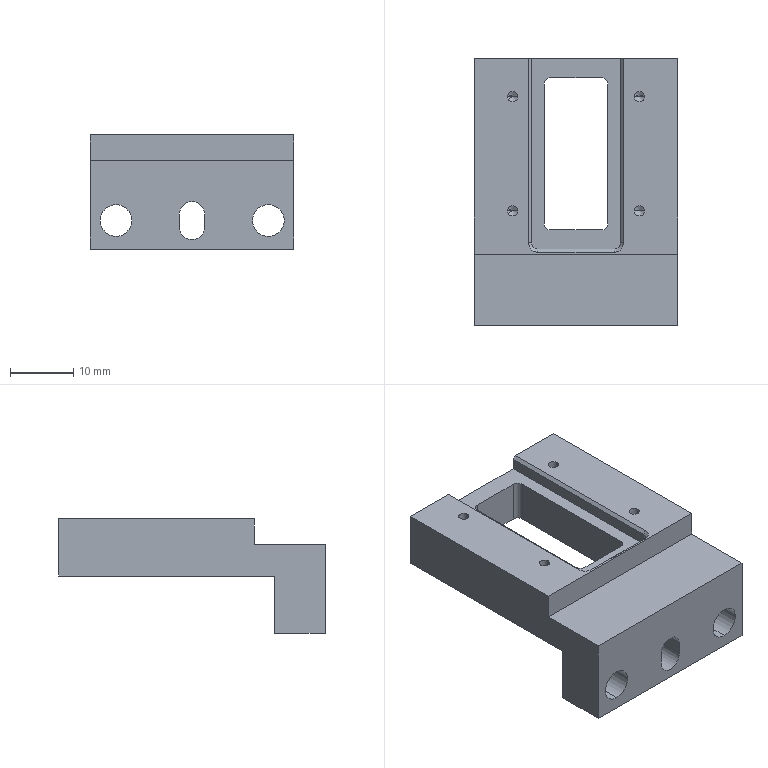Part | 1 solid | 54 faces | box 32 x 42 x 18 mm | volume 9868 mm3 | plane 23 | cylinder 21 | cone 10 | commonest cylinder face diameters 1.6 x8 2 x6 5 x4 4 x3
STEP:
#1=CARTESIAN_POINT('',(9.2,-8.591,-5.2));
#2=VERTEX_POINT('',#1);
#3=CARTESIAN_POINT('',(10.8,-8.591,-5.2));
#4=VERTEX_POINT('',#3);
#5=CARTESIAN_POINT('',(10.,-8.591,-5.2));
#6=DIRECTION('',(0.,0.,1.));
#7=DIRECTION('',(1.,0.,0.));
#8=AXIS2_PLACEMENT_3D('',#5,#6,#7);
#9=CIRCLE('',#8,0.8);
#10=EDGE_CURVE('',#2,#4,#9,.T.);
#11=ORIENTED_EDGE('',*,*,#10,.F.);
#12=CARTESIAN_POINT('',(9.2,-8.591,0.));
#13=VERTEX_POINT('',#12);
#14=CARTESIAN_POINT('',(9.2,-8.591,0.));
#15=DIRECTION('',(0.,0.,1.));
#16=VECTOR('',#15,1000.);
#17=LINE('',#14,#16);
#18=EDGE_CURVE('',#13,#2,#17,.F.);
#19=ORIENTED_EDGE('',*,*,#18,.F.);
#20=CARTESIAN_POINT('',(10.8,-8.591,0.));
#21=VERTEX_POINT('',#20);
#22=CARTESIAN_POINT('',(10.,-8.591,0.));
#23=DIRECTION('',(0.,0.,1.));
#24=DIRECTION('',(1.,0.,0.));
#25=AXIS2_PLACEMENT_3D('',#22,#23,#24);
#26=CIRCLE('',#25,0.8);
#27=EDGE_CURVE('',#13,#21,#26,.T.);
#28=ORIENTED_EDGE('',*,*,#27,.T.);
#29=CARTESIAN_POINT('',(10.8,-8.591,0.));
#30=DIRECTION('',(0.,0.,1.));
#31=VECTOR('',#30,1000.);
#32=LINE('',#29,#31);
#33=EDGE_CURVE('',#21,#4,#32,.F.);
#34=ORIENTED_EDGE('',*,*,#33,.T.);
#35=EDGE_LOOP('',(#11,#19,#28,#34));
#36=FACE_BOUND('',#35,.T.);
#37=CARTESIAN_POINT('',(10.,-8.591,0.));
#38=DIRECTION('',(0.,0.,1.));
#39=DIRECTION('',(-1.,0.,0.));
#40=AXIS2_PLACEMENT_3D('',#37,#38,#39);
#41=CYLINDRICAL_SURFACE('',#40,0.8);
#42=ADVANCED_FACE('',(#36),#41,.F.);
#43=CARTESIAN_POINT('',(10.,-8.591,-5.681));
#44=VERTEX_POINT('',#43);
#45=CARTESIAN_POINT('',(10.8,-8.591,-5.2));
#46=DIRECTION('',(0.8572,0.,0.515));
#47=VECTOR('',#46,1000.);
#48=LINE('',#45,#47);
#49=EDGE_CURVE('',#4,#44,#48,.F.);
#50=ORIENTED_EDGE('',*,*,#49,.T.);
#51=CARTESIAN_POINT('',(9.2,-8.591,-5.2));
#52=DIRECTION('',(-0.8572,0.,0.515));
#53=VECTOR('',#52,1000.);
#54=LINE('',#51,#53);
#55=EDGE_CURVE('',#2,#44,#54,.F.);
#56=ORIENTED_EDGE('',*,*,#55,.F.);
#57=ORIENTED_EDGE('',*,*,#10,.T.);
#58=EDGE_LOOP('',(#50,#56,#57));
#59=FACE_BOUND('',#58,.T.);
#60=CARTESIAN_POINT('',(10.,-8.591,-5.2));
#61=DIRECTION('',(0.,0.,1.));
#62=DIRECTION('',(-1.,0.,0.));
#63=AXIS2_PLACEMENT_3D('',#60,#61,#62);
#64=CONICAL_SURFACE('',#63,0.8,1.03);
#65=ADVANCED_FACE('',(#59),#64,.F.);
#66=CARTESIAN_POINT('',(-10.8,-8.591,-5.2));
#67=VERTEX_POINT('',#66);
#68=CARTESIAN_POINT('',(-9.2,-8.591,-5.2));
#69=VERTEX_POINT('',#68);
#70=CARTESIAN_POINT('',(-10.,-8.591,-5.2));
#71=DIRECTION('',(0.,0.,1.));
#72=DIRECTION('',(1.,0.,0.));
#73=AXIS2_PLACEMENT_3D('',#70,#71,#72);
#74=CIRCLE('',#73,0.8);
#75=EDGE_CURVE('',#67,#69,#74,.T.);
#76=ORIENTED_EDGE('',*,*,#75,.F.);
#77=CARTESIAN_POINT('',(-10.8,-8.591,0.));
#78=VERTEX_POINT('',#77);
#79=CARTESIAN_POINT('',(-10.8,-8.591,0.));
#80=DIRECTION('',(0.,0.,1.));
#81=VECTOR('',#80,1000.);
#82=LINE('',#79,#81);
#83=EDGE_CURVE('',#78,#67,#82,.F.);
#84=ORIENTED_EDGE('',*,*,#83,.F.);
#85=CARTESIAN_POINT('',(-9.2,-8.591,0.));
#86=VERTEX_POINT('',#85);
#87=CARTESIAN_POINT('',(-10.,-8.591,0.));
#88=DIRECTION('',(0.,0.,1.));
#89=DIRECTION('',(1.,0.,0.));
#90=AXIS2_PLACEMENT_3D('',#87,#88,#89);
#91=CIRCLE('',#90,0.8);
#92=EDGE_CURVE('',#78,#86,#91,.T.);
#93=ORIENTED_EDGE('',*,*,#92,.T.);
#94=CARTESIAN_POINT('',(-9.2,-8.591,0.));
#95=DIRECTION('',(0.,0.,1.));
#96=VECTOR('',#95,1000.);
#97=LINE('',#94,#96);
#98=EDGE_CURVE('',#86,#69,#97,.F.);
#99=ORIENTED_EDGE('',*,*,#98,.T.);
#100=EDGE_LOOP('',(#76,#84,#93,#99));
#101=FACE_BOUND('',#100,.T.);
#102=CARTESIAN_POINT('',(-10.,-8.591,0.));
#103=DIRECTION('',(0.,0.,1.));
#104=DIRECTION('',(-1.,0.,0.));
#105=AXIS2_PLACEMENT_3D('',#102,#103,#104);
#106=CYLINDRICAL_SURFACE('',#105,0.8);
#107=ADVANCED_FACE('',(#101),#106,.F.);
#108=CARTESIAN_POINT('',(-10.,-8.591,-5.681));
#109=VERTEX_POINT('',#108);
#110=CARTESIAN_POINT('',(-9.2,-8.591,-5.2));
#111=DIRECTION('',(0.8572,0.,0.515));
#112=VECTOR('',#111,1000.);
#113=LINE('',#110,#112);
#114=EDGE_CURVE('',#69,#109,#113,.F.);
#115=ORIENTED_EDGE('',*,*,#114,.T.);
#116=CARTESIAN_POINT('',(-10.8,-8.591,-5.2));
#117=DIRECTION('',(-0.8572,0.,0.515));
#118=VECTOR('',#117,1000.);
#119=LINE('',#116,#118);
#120=EDGE_CURVE('',#67,#109,#119,.F.);
#121=ORIENTED_EDGE('',*,*,#120,.F.);
#122=ORIENTED_EDGE('',*,*,#75,.T.);
#123=EDGE_LOOP('',(#115,#121,#122));
#124=FACE_BOUND('',#123,.T.);
#125=CARTESIAN_POINT('',(-10.,-8.591,-5.2));
#126=DIRECTION('',(0.,0.,1.));
#127=DIRECTION('',(-1.,0.,0.));
#128=AXIS2_PLACEMENT_3D('',#125,#126,#127);
#129=CONICAL_SURFACE('',#128,0.8,1.03);
#130=ADVANCED_FACE('',(#124),#129,.F.);
#131=CARTESIAN_POINT('',(9.2,9.409,-5.2));
#132=VERTEX_POINT('',#131);
#133=CARTESIAN_POINT('',(10.8,9.409,-5.2));
#134=VERTEX_POINT('',#133);
#135=CARTESIAN_POINT('',(10.,9.409,-5.2));
#136=DIRECTION('',(0.,0.,1.));
#137=DIRECTION('',(1.,0.,0.));
#138=AXIS2_PLACEMENT_3D('',#135,#136,#137);
#139=CIRCLE('',#138,0.8);
#140=EDGE_CURVE('',#132,#134,#139,.T.);
#141=ORIENTED_EDGE('',*,*,#140,.F.);
#142=CARTESIAN_POINT('',(9.2,9.409,0.));
#143=VERTEX_POINT('',#142);
#144=CARTESIAN_POINT('',(9.2,9.409,0.));
#145=DIRECTION('',(0.,0.,1.));
#146=VECTOR('',#145,1000.);
#147=LINE('',#144,#146);
#148=EDGE_CURVE('',#143,#132,#147,.F.);
#149=ORIENTED_EDGE('',*,*,#148,.F.);
#150=CARTESIAN_POINT('',(10.8,9.409,0.));
#151=VERTEX_POINT('',#150);
#152=CARTESIAN_POINT('',(10.,9.409,0.));
#153=DIRECTION('',(0.,0.,1.));
#154=DIRECTION('',(1.,0.,0.));
#155=AXIS2_PLACEMENT_3D('',#152,#153,#154);
#156=CIRCLE('',#155,0.8);
#157=EDGE_CURVE('',#143,#151,#156,.T.);
#158=ORIENTED_EDGE('',*,*,#157,.T.);
#159=CARTESIAN_POINT('',(10.8,9.409,0.));
#160=DIRECTION('',(0.,0.,1.));
#161=VECTOR('',#160,1000.);
#162=LINE('',#159,#161);
#163=EDGE_CURVE('',#151,#134,#162,.F.);
#164=ORIENTED_EDGE('',*,*,#163,.T.);
#165=EDGE_LOOP('',(#141,#149,#158,#164));
#166=FACE_BOUND('',#165,.T.);
#167=CARTESIAN_POINT('',(10.,9.409,0.));
#168=DIRECTION('',(0.,0.,1.));
#169=DIRECTION('',(-1.,0.,0.));
#170=AXIS2_PLACEMENT_3D('',#167,#168,#169);
#171=CYLINDRICAL_SURFACE('',#170,0.8);
#172=ADVANCED_FACE('',(#166),#171,.F.);
#173=CARTESIAN_POINT('',(10.,9.409,-5.681));
#174=VERTEX_POINT('',#173);
#175=CARTESIAN_POINT('',(10.8,9.409,-5.2));
#176=DIRECTION('',(0.8572,0.,0.515));
#177=VECTOR('',#176,1000.);
#178=LINE('',#175,#177);
#179=EDGE_CURVE('',#134,#174,#178,.F.);
#180=ORIENTED_EDGE('',*,*,#179,.T.);
#181=CARTESIAN_POINT('',(9.2,9.409,-5.2));
#182=DIRECTION('',(-0.8572,0.,0.515));
#183=VECTOR('',#182,1000.);
#184=LINE('',#181,#183);
#185=EDGE_CURVE('',#132,#174,#184,.F.);
#186=ORIENTED_EDGE('',*,*,#185,.F.);
#187=ORIENTED_EDGE('',*,*,#140,.T.);
#188=EDGE_LOOP('',(#180,#186,#187));
#189=FACE_BOUND('',#188,.T.);
#190=CARTESIAN_POINT('',(10.,9.409,-5.2));
#191=DIRECTION('',(0.,0.,1.));
#192=DIRECTION('',(-1.,0.,0.));
#193=AXIS2_PLACEMENT_3D('',#190,#191,#192);
#194=CONICAL_SURFACE('',#193,0.8,1.03);
#195=ADVANCED_FACE('',(#189),#194,.F.);
#196=CARTESIAN_POINT('',(-10.8,9.409,-5.2));
#197=VERTEX_POINT('',#196);
#198=CARTESIAN_POINT('',(-9.2,9.409,-5.2));
#199=VERTEX_POINT('',#198);
#200=CARTESIAN_POINT('',(-10.,9.409,-5.2));
#201=DIRECTION('',(0.,0.,1.));
#202=DIRECTION('',(1.,0.,0.));
#203=AXIS2_PLACEMENT_3D('',#200,#201,#202);
#204=CIRCLE('',#203,0.8);
#205=EDGE_CURVE('',#197,#199,#204,.T.);
#206=ORIENTED_EDGE('',*,*,#205,.F.);
#207=CARTESIAN_POINT('',(-10.8,9.409,0.));
#208=VERTEX_POINT('',#207);
#209=CARTESIAN_POINT('',(-10.8,9.409,0.));
#210=DIRECTION('',(0.,0.,1.));
#211=VECTOR('',#210,1000.);
#212=LINE('',#209,#211);
#213=EDGE_CURVE('',#208,#197,#212,.F.);
#214=ORIENTED_EDGE('',*,*,#213,.F.);
#215=CARTESIAN_POINT('',(-9.2,9.409,0.));
#216=VERTEX_POINT('',#215);
#217=CARTESIAN_POINT('',(-10.,9.409,0.));
#218=DIRECTION('',(0.,0.,1.));
#219=DIRECTION('',(1.,0.,0.));
#220=AXIS2_PLACEMENT_3D('',#217,#218,#219);
#221=CIRCLE('',#220,0.8);
#222=EDGE_CURVE('',#208,#216,#221,.T.);
#223=ORIENTED_EDGE('',*,*,#222,.T.);
#224=CARTESIAN_POINT('',(-9.2,9.409,0.));
#225=DIRECTION('',(0.,0.,1.));
#226=VECTOR('',#225,1000.);
#227=LINE('',#224,#226);
#228=EDGE_CURVE('',#216,#199,#227,.F.);
#229=ORIENTED_EDGE('',*,*,#228,.T.);
#230=EDGE_LOOP('',(#206,#214,#223,#229));
#231=FACE_BOUND('',#230,.T.);
#232=CARTESIAN_POINT('',(-10.,9.409,0.));
#233=DIRECTION('',(0.,0.,1.));
#234=DIRECTION('',(-1.,0.,0.));
#235=AXIS2_PLACEMENT_3D('',#232,#233,#234);
#236=CYLINDRICAL_SURFACE('',#235,0.8);
#237=ADVANCED_FACE('',(#231),#236,.F.);
#238=CARTESIAN_POINT('',(-10.,9.409,-5.681));
#239=VERTEX_POINT('',#238);
#240=CARTESIAN_POINT('',(-9.2,9.409,-5.2));
#241=DIRECTION('',(0.8572,0.,0.515));
#242=VECTOR('',#241,1000.);
#243=LINE('',#240,#242);
#244=EDGE_CURVE('',#199,#239,#243,.F.);
#245=ORIENTED_EDGE('',*,*,#244,.T.);
#246=CARTESIAN_POINT('',(-10.8,9.409,-5.2));
#247=DIRECTION('',(-0.8572,0.,0.515));
#248=VECTOR('',#247,1000.);
#249=LINE('',#246,#248);
#250=EDGE_CURVE('',#197,#239,#249,.F.);
#251=ORIENTED_EDGE('',*,*,#250,.F.);
#252=ORIENTED_EDGE('',*,*,#205,.T.);
#253=EDGE_LOOP('',(#245,#251,#252));
#254=FACE_BOUND('',#253,.T.);
#255=CARTESIAN_POINT('',(-10.,9.409,-5.2));
#256=DIRECTION('',(0.,0.,1.));
#257=DIRECTION('',(-1.,0.,0.));
#258=AXIS2_PLACEMENT_3D('',#255,#256,#257);
#259=CONICAL_SURFACE('',#258,0.8,1.03);
#260=ADVANCED_FACE('',(#254),#259,.F.);
#261=CARTESIAN_POINT('',(0.,-18.6,-10.5));
#262=VERTEX_POINT('',#261);
#263=CARTESIAN_POINT('',(-2.,-18.6,-12.5));
#264=VERTEX_POINT('',#263);
#265=CARTESIAN_POINT('',(0.,-18.6,-12.5));
#266=DIRECTION('',(0.,-1.,0.));
#267=DIRECTION('',(0.,0.,1.));
#268=AXIS2_PLACEMENT_3D('',#265,#266,#267);
#269=CIRCLE('',#268,2.);
#270=EDGE_CURVE('',#262,#264,#269,.T.);
#271=ORIENTED_EDGE('',*,*,#270,.F.);
#272=CARTESIAN_POINT('',(0.,-26.6,-10.5));
#273=VERTEX_POINT('',#272);
#274=CARTESIAN_POINT('',(0.,-16.6,-10.5));
#275=DIRECTION('',(0.,-1.,0.));
#276=VECTOR('',#275,1000.);
#277=LINE('',#274,#276);
#278=EDGE_CURVE('',#262,#273,#277,.T.);
#279=ORIENTED_EDGE('',*,*,#278,.T.);
#280=CARTESIAN_POINT('',(-2.,-26.6,-12.5));
#281=VERTEX_POINT('',#280);
#282=CARTESIAN_POINT('',(0.,-26.6,-12.5));
#283=DIRECTION('',(0.,-1.,0.));
#284=DIRECTION('',(0.,0.,1.));
#285=AXIS2_PLACEMENT_3D('',#282,#283,#284);
#286=CIRCLE('',#285,2.);
#287=EDGE_CURVE('',#273,#281,#286,.T.);
#288=ORIENTED_EDGE('',*,*,#287,.T.);
#289=CARTESIAN_POINT('',(-2.,-16.6,-12.5));
#290=DIRECTION('',(0.,-1.,0.));
#291=VECTOR('',#290,1000.);
#292=LINE('',#289,#291);
#293=EDGE_CURVE('',#264,#281,#292,.T.);
#294=ORIENTED_EDGE('',*,*,#293,.F.);
#295=EDGE_LOOP('',(#271,#279,#288,#294));
#296=FACE_BOUND('',#295,.T.);
#297=CARTESIAN_POINT('',(0.,-16.6,-12.5));
#298=DIRECTION('',(0.,-1.,0.));
#299=DIRECTION('',(0.,0.,-1.));
#300=AXIS2_PLACEMENT_3D('',#297,#298,#299);
#301=CYLINDRICAL_SURFACE('',#300,2.);
#302=ADVANCED_FACE('',(#296),#301,.F.);
#303=CARTESIAN_POINT('',(-11.974,-26.6,-11.));
#304=VERTEX_POINT('',#303);
#305=CARTESIAN_POINT('',(-11.974,-26.6,-16.));
#306=VERTEX_POINT('',#305);
#307=CARTESIAN_POINT('',(-11.974,-26.6,-13.5));
#308=DIRECTION('',(0.,1.,0.));
#309=DIRECTION('',(0.,0.,-1.));
#310=AXIS2_PLACEMENT_3D('',#307,#308,#309);
#311=CIRCLE('',#310,2.5);
#312=EDGE_CURVE('',#304,#306,#311,.T.);
#313=ORIENTED_EDGE('',*,*,#312,.F.);
#314=CARTESIAN_POINT('',(-11.974,-18.6,-11.));
#315=VERTEX_POINT('',#314);
#316=CARTESIAN_POINT('',(-11.974,-18.6,-11.));
#317=DIRECTION('',(0.,1.,0.));
#318=VECTOR('',#317,1000.);
#319=LINE('',#316,#318);
#320=EDGE_CURVE('',#315,#304,#319,.F.);
#321=ORIENTED_EDGE('',*,*,#320,.F.);
#322=CARTESIAN_POINT('',(-11.974,-18.6,-16.));
#323=VERTEX_POINT('',#322);
#324=CARTESIAN_POINT('',(-11.974,-18.6,-13.5));
#325=DIRECTION('',(0.,1.,0.));
#326=DIRECTION('',(0.,0.,-1.));
#327=AXIS2_PLACEMENT_3D('',#324,#325,#326);
#328=CIRCLE('',#327,2.5);
#329=EDGE_CURVE('',#315,#323,#328,.T.);
#330=ORIENTED_EDGE('',*,*,#329,.T.);
#331=CARTESIAN_POINT('',(-11.974,-18.6,-16.));
#332=DIRECTION('',(0.,1.,0.));
#333=VECTOR('',#332,1000.);
#334=LINE('',#331,#333);
#335=EDGE_CURVE('',#323,#306,#334,.F.);
#336=ORIENTED_EDGE('',*,*,#335,.T.);
#337=EDGE_LOOP('',(#313,#321,#330,#336));
#338=FACE_BOUND('',#337,.T.);
#339=CARTESIAN_POINT('',(-11.974,-18.6,-13.5));
#340=DIRECTION('',(0.,1.,0.));
#341=DIRECTION('',(0.,0.,1.));
#342=AXIS2_PLACEMENT_3D('',#339,#340,#341);
#343=CYLINDRICAL_SURFACE('',#342,2.5);
#344=ADVANCED_FACE('',(#338),#343,.F.);
#345=CARTESIAN_POINT('',(12.026,-26.6,-11.));
#346=VERTEX_POINT('',#345);
#347=CARTESIAN_POINT('',(12.026,-26.6,-16.));
#348=VERTEX_POINT('',#347);
#349=CARTESIAN_POINT('',(12.026,-26.6,-13.5));
#350=DIRECTION('',(0.,1.,0.));
#351=DIRECTION('',(0.,0.,-1.));
#352=AXIS2_PLACEMENT_3D('',#349,#350,#351);
#353=CIRCLE('',#352,2.5);
#354=EDGE_CURVE('',#346,#348,#353,.T.);
#355=ORIENTED_EDGE('',*,*,#354,.F.);
#356=CARTESIAN_POINT('',(12.026,-18.6,-11.));
#357=VERTEX_POINT('',#356);
#358=CARTESIAN_POINT('',(12.026,-18.6,-11.));
#359=DIRECTION('',(0.,1.,0.));
#360=VECTOR('',#359,1000.);
#361=LINE('',#358,#360);
#362=EDGE_CURVE('',#357,#346,#361,.F.);
#363=ORIENTED_EDGE('',*,*,#362,.F.);
#364=CARTESIAN_POINT('',(12.026,-18.6,-16.));
#365=VERTEX_POINT('',#364);
#366=CARTESIAN_POINT('',(12.026,-18.6,-13.5));
#367=DIRECTION('',(0.,1.,0.));
#368=DIRECTION('',(0.,0.,-1.));
#369=AXIS2_PLACEMENT_3D('',#366,#367,#368);
#370=CIRCLE('',#369,2.5);
#371=EDGE_CURVE('',#357,#365,#370,.T.);
#372=ORIENTED_EDGE('',*,*,#371,.T.);
#373=CARTESIAN_POINT('',(12.026,-18.6,-16.));
#374=DIRECTION('',(0.,1.,0.));
#375=VECTOR('',#374,1000.);
#376=LINE('',#373,#375);
#377=EDGE_CURVE('',#365,#348,#376,.F.);
#378=ORIENTED_EDGE('',*,*,#377,.T.);
#379=EDGE_LOOP('',(#355,#363,#372,#378));
#380=FACE_BOUND('',#379,.T.);
#381=CARTESIAN_POINT('',(12.026,-18.6,-13.5));
#382=DIRECTION('',(0.,1.,0.));
#383=DIRECTION('',(0.,0.,1.));
#384=AXIS2_PLACEMENT_3D('',#381,#382,#383);
#385=CYLINDRICAL_SURFACE('',#384,2.5);
#386=ADVANCED_FACE('',(#380),#385,.F.);
#387=CARTESIAN_POINT('',(16.,-18.6,-18.));
#388=VERTEX_POINT('',#387);
#389=CARTESIAN_POINT('',(16.,-18.6,-9.));
#390=VERTEX_POINT('',#389);
#391=CARTESIAN_POINT('',(16.,-18.6,-18.));
#392=DIRECTION('',(0.,0.,1.));
#393=VECTOR('',#392,1000.);
#394=LINE('',#391,#393);
#395=EDGE_CURVE('',#388,#390,#394,.T.);
#396=ORIENTED_EDGE('',*,*,#395,.T.);
#397=CARTESIAN_POINT('',(16.,15.4,-9.));
#398=VERTEX_POINT('',#397);
#399=CARTESIAN_POINT('',(16.,15.4,-9.));
#400=DIRECTION('',(0.,1.,0.));
#401=VECTOR('',#400,1000.);
#402=LINE('',#399,#401);
#403=EDGE_CURVE('',#390,#398,#402,.T.);
#404=ORIENTED_EDGE('',*,*,#403,.T.);
#405=CARTESIAN_POINT('',(16.,15.4,0.));
#406=VERTEX_POINT('',#405);
#407=CARTESIAN_POINT('',(16.,15.4,-18.));
#408=DIRECTION('',(0.,0.,-1.));
#409=VECTOR('',#408,1000.);
#410=LINE('',#407,#409);
#411=EDGE_CURVE('',#406,#398,#410,.T.);
#412=ORIENTED_EDGE('',*,*,#411,.F.);
#413=CARTESIAN_POINT('',(16.,-15.4,0.));
#414=VERTEX_POINT('',#413);
#415=CARTESIAN_POINT('',(16.,15.4,0.));
#416=DIRECTION('',(0.,-1.,0.));
#417=VECTOR('',#416,1000.);
#418=LINE('',#415,#417);
#419=EDGE_CURVE('',#406,#414,#418,.T.);
#420=ORIENTED_EDGE('',*,*,#419,.T.);
#421=CARTESIAN_POINT('',(16.,-15.4,-4.));
#422=VERTEX_POINT('',#421);
#423=CARTESIAN_POINT('',(16.,-15.4,0.));
#424=DIRECTION('',(0.,0.,-1.));
#425=VECTOR('',#424,1000.);
#426=LINE('',#423,#425);
#427=EDGE_CURVE('',#414,#422,#426,.T.);
#428=ORIENTED_EDGE('',*,*,#427,.T.);
#429=CARTESIAN_POINT('',(16.,-26.6,-4.));
#430=VERTEX_POINT('',#429);
#431=CARTESIAN_POINT('',(16.,-26.6,-4.));
#432=DIRECTION('',(0.,-1.,0.));
#433=VECTOR('',#432,1000.);
#434=LINE('',#431,#433);
#435=EDGE_CURVE('',#422,#430,#434,.T.);
#436=ORIENTED_EDGE('',*,*,#435,.T.);
#437=CARTESIAN_POINT('',(16.,-26.6,-18.));
#438=VERTEX_POINT('',#437);
#439=CARTESIAN_POINT('',(16.,-26.6,-18.));
#440=DIRECTION('',(0.,0.,-1.));
#441=VECTOR('',#440,1000.);
#442=LINE('',#439,#441);
#443=EDGE_CURVE('',#430,#438,#442,.T.);
#444=ORIENTED_EDGE('',*,*,#443,.T.);
#445=CARTESIAN_POINT('',(16.,15.4,-18.));
#446=DIRECTION('',(0.,-1.,0.));
#447=VECTOR('',#446,1000.);
#448=LINE('',#445,#447);
#449=EDGE_CURVE('',#388,#438,#448,.T.);
#450=ORIENTED_EDGE('',*,*,#449,.F.);
#451=EDGE_LOOP('',(#396,#404,#412,#420,#428,#436,#444,#450));
#452=FACE_BOUND('',#451,.T.);
#453=CARTESIAN_POINT('',(16.,15.4,-18.));
#454=DIRECTION('',(-1.,0.,0.));
#455=DIRECTION('',(0.,0.,-1.));
#456=AXIS2_PLACEMENT_3D('',#453,#454,#455);
#457=PLANE('',#456);
#458=ADVANCED_FACE('',(#452),#457,.F.);
#459=CARTESIAN_POINT('',(-16.,-18.6,-18.));
#460=VERTEX_POINT('',#459);
#461=CARTESIAN_POINT('',(-16.,-26.6,-18.));
#462=VERTEX_POINT('',#461);
#463=CARTESIAN_POINT('',(-16.,15.4,-18.));
#464=DIRECTION('',(0.,-1.,0.));
#465=VECTOR('',#464,1000.);
#466=LINE('',#463,#465);
#467=EDGE_CURVE('',#460,#462,#466,.T.);
#468=ORIENTED_EDGE('',*,*,#467,.F.);
#469=CARTESIAN_POINT('',(16.,-18.6,-18.));
#470=DIRECTION('',(-1.,0.,0.));
#471=VECTOR('',#470,1000.);
#472=LINE('',#469,#471);
#473=EDGE_CURVE('',#388,#460,#472,.T.);
#474=ORIENTED_EDGE('',*,*,#473,.F.);
#475=ORIENTED_EDGE('',*,*,#449,.T.);
#476=CARTESIAN_POINT('',(-16.,-26.6,-18.));
#477=DIRECTION('',(-1.,0.,0.));
#478=VECTOR('',#477,1000.);
#479=LINE('',#476,#478);
#480=EDGE_CURVE('',#438,#462,#479,.T.);
#481=ORIENTED_EDGE('',*,*,#480,.T.);
#482=EDGE_LOOP('',(#468,#474,#475,#481));
#483=FACE_BOUND('',#482,.T.);
#484=CARTESIAN_POINT('',(-16.,15.4,-18.));
#485=DIRECTION('',(0.,0.,1.));
#486=DIRECTION('',(-1.,0.,0.));
#487=AXIS2_PLACEMENT_3D('',#484,#485,#486);
#488=PLANE('',#487);
#489=ADVANCED_FACE('',(#483),#488,.F.);
#490=CARTESIAN_POINT('',(-16.,15.4,-9.));
#491=VERTEX_POINT('',#490);
#492=CARTESIAN_POINT('',(-16.,15.4,0.));
#493=VERTEX_POINT('',#492);
#494=CARTESIAN_POINT('',(-16.,15.4,-18.));
#495=DIRECTION('',(0.,0.,1.));
#496=VECTOR('',#495,1000.);
#497=LINE('',#494,#496);
#498=EDGE_CURVE('',#491,#493,#497,.T.);
#499=ORIENTED_EDGE('',*,*,#498,.F.);
#500=CARTESIAN_POINT('',(-16.,-18.6,-9.));
#501=VERTEX_POINT('',#500);
#502=CARTESIAN_POINT('',(-16.,15.4,-9.));
#503=DIRECTION('',(0.,1.,0.));
#504=VECTOR('',#503,1000.);
#505=LINE('',#502,#504);
#506=EDGE_CURVE('',#501,#491,#505,.T.);
#507=ORIENTED_EDGE('',*,*,#506,.F.);
#508=CARTESIAN_POINT('',(-16.,-18.6,-18.));
#509=DIRECTION('',(0.,0.,1.));
#510=VECTOR('',#509,1000.);
#511=LINE('',#508,#510);
#512=EDGE_CURVE('',#460,#501,#511,.T.);
#513=ORIENTED_EDGE('',*,*,#512,.F.);
#514=ORIENTED_EDGE('',*,*,#467,.T.);
#515=CARTESIAN_POINT('',(-16.,-26.6,-4.));
#516=VERTEX_POINT('',#515);
#517=CARTESIAN_POINT('',(-16.,-26.6,-18.));
#518=DIRECTION('',(0.,0.,1.));
#519=VECTOR('',#518,1000.);
#520=LINE('',#517,#519);
#521=EDGE_CURVE('',#462,#516,#520,.T.);
#522=ORIENTED_EDGE('',*,*,#521,.T.);
#523=CARTESIAN_POINT('',(-16.,-15.4,-4.));
#524=VERTEX_POINT('',#523);
#525=CARTESIAN_POINT('',(-16.,-26.6,-4.));
#526=DIRECTION('',(0.,-1.,0.));
#527=VECTOR('',#526,1000.);
#528=LINE('',#525,#527);
#529=EDGE_CURVE('',#524,#516,#528,.T.);
#530=ORIENTED_EDGE('',*,*,#529,.F.);
#531=CARTESIAN_POINT('',(-16.,-15.4,0.));
#532=VERTEX_POINT('',#531);
#533=CARTESIAN_POINT('',(-16.,-15.4,0.));
#534=DIRECTION('',(0.,0.,-1.));
#535=VECTOR('',#534,1000.);
#536=LINE('',#533,#535);
#537=EDGE_CURVE('',#532,#524,#536,.T.);
#538=ORIENTED_EDGE('',*,*,#537,.F.);
#539=CARTESIAN_POINT('',(-16.,15.4,0.));
#540=DIRECTION('',(0.,-1.,0.));
#541=VECTOR('',#540,1000.);
#542=LINE('',#539,#541);
#543=EDGE_CURVE('',#493,#532,#542,.T.);
#544=ORIENTED_EDGE('',*,*,#543,.F.);
#545=EDGE_LOOP('',(#499,#507,#513,#514,#522,#530,#538,#544));
#546=FACE_BOUND('',#545,.T.);
#547=CARTESIAN_POINT('',(-16.,15.4,-18.));
#548=DIRECTION('',(1.,0.,0.));
#549=DIRECTION('',(0.,0.,1.));
#550=AXIS2_PLACEMENT_3D('',#547,#548,#549);
#551=PLANE('',#550);
#552=ADVANCED_FACE('',(#546),#551,.F.);
#553=CARTESIAN_POINT('',(10.,-8.591,0.));
#554=DIRECTION('',(0.,0.,1.));
#555=DIRECTION('',(1.,0.,0.));
#556=AXIS2_PLACEMENT_3D('',#553,#554,#555);
#557=CIRCLE('',#556,0.8);
#558=EDGE_CURVE('',#21,#13,#557,.T.);
#559=ORIENTED_EDGE('',*,*,#558,.F.);
#560=ORIENTED_EDGE('',*,*,#27,.F.);
#561=EDGE_LOOP('',(#559,#560));
#562=FACE_BOUND('',#561,.T.);
#563=CARTESIAN_POINT('',(-10.,-8.591,0.));
#564=DIRECTION('',(0.,0.,1.));
#565=DIRECTION('',(1.,0.,0.));
#566=AXIS2_PLACEMENT_3D('',#563,#564,#565);
#567=CIRCLE('',#566,0.8);
#568=EDGE_CURVE('',#86,#78,#567,.T.);
#569=ORIENTED_EDGE('',*,*,#568,.F.);
#570=ORIENTED_EDGE('',*,*,#92,.F.);
#571=EDGE_LOOP('',(#569,#570));
#572=FACE_BOUND('',#571,.T.);
#573=CARTESIAN_POINT('',(10.,9.409,0.));
#574=DIRECTION('',(0.,0.,1.));
#575=DIRECTION('',(1.,0.,0.));
#576=AXIS2_PLACEMENT_3D('',#573,#574,#575);
#577=CIRCLE('',#576,0.8);
#578=EDGE_CURVE('',#151,#143,#577,.T.);
#579=ORIENTED_EDGE('',*,*,#578,.F.);
#580=ORIENTED_EDGE('',*,*,#157,.F.);
#581=EDGE_LOOP('',(#579,#580));
#582=FACE_BOUND('',#581,.T.);
#583=CARTESIAN_POINT('',(-10.,9.409,0.));
#584=DIRECTION('',(0.,0.,1.));
#585=DIRECTION('',(1.,0.,0.));
#586=AXIS2_PLACEMENT_3D('',#583,#584,#585);
#587=CIRCLE('',#586,0.8);
#588=EDGE_CURVE('',#216,#208,#587,.T.);
#589=ORIENTED_EDGE('',*,*,#588,.F.);
#590=ORIENTED_EDGE('',*,*,#222,.F.);
#591=EDGE_LOOP('',(#589,#590));
#592=FACE_BOUND('',#591,.T.);
#593=CARTESIAN_POINT('',(-6.,-15.1,0.));
#594=VERTEX_POINT('',#593);
#595=CARTESIAN_POINT('',(-7.5,-13.6,0.));
#596=VERTEX_POINT('',#595);
#597=CARTESIAN_POINT('',(-6.,-13.6,0.));
#598=DIRECTION('',(0.,0.,-1.));
#599=DIRECTION('',(-1.,0.,0.));
#600=AXIS2_PLACEMENT_3D('',#597,#598,#599);
#601=CIRCLE('',#600,1.5);
#602=EDGE_CURVE('',#594,#596,#601,.T.);
#603=ORIENTED_EDGE('',*,*,#602,.T.);
#604=CARTESIAN_POINT('',(-7.5,15.4,0.));
#605=VERTEX_POINT('',#604);
#606=CARTESIAN_POINT('',(-7.5,15.4,0.));
#607=DIRECTION('',(0.,1.,0.));
#608=VECTOR('',#607,1000.);
#609=LINE('',#606,#608);
#610=EDGE_CURVE('',#596,#605,#609,.T.);
#611=ORIENTED_EDGE('',*,*,#610,.T.);
#612=CARTESIAN_POINT('',(-16.,15.4,0.));
#613=DIRECTION('',(1.,0.,0.));
#614=VECTOR('',#613,1000.);
#615=LINE('',#612,#614);
#616=EDGE_CURVE('',#493,#605,#615,.T.);
#617=ORIENTED_EDGE('',*,*,#616,.F.);
#618=ORIENTED_EDGE('',*,*,#543,.T.);
#619=CARTESIAN_POINT('',(16.,-15.4,0.));
#620=DIRECTION('',(-1.,0.,0.));
#621=VECTOR('',#620,1000.);
#622=LINE('',#619,#621);
#623=EDGE_CURVE('',#414,#532,#622,.T.);
#624=ORIENTED_EDGE('',*,*,#623,.F.);
#625=ORIENTED_EDGE('',*,*,#419,.F.);
#626=CARTESIAN_POINT('',(7.5,15.4,0.));
#627=VERTEX_POINT('',#626);
#628=CARTESIAN_POINT('',(-16.,15.4,0.));
#629=DIRECTION('',(1.,0.,0.));
#630=VECTOR('',#629,1000.);
#631=LINE('',#628,#630);
#632=EDGE_CURVE('',#627,#406,#631,.T.);
#633=ORIENTED_EDGE('',*,*,#632,.F.);
#634=CARTESIAN_POINT('',(7.5,-13.6,0.));
#635=VERTEX_POINT('',#634);
#636=CARTESIAN_POINT('',(7.5,15.4,0.));
#637=DIRECTION('',(0.,-1.,0.));
#638=VECTOR('',#637,1000.);
#639=LINE('',#636,#638);
#640=EDGE_CURVE('',#627,#635,#639,.T.);
#641=ORIENTED_EDGE('',*,*,#640,.T.);
#642=CARTESIAN_POINT('',(6.,-15.1,0.));
#643=VERTEX_POINT('',#642);
#644=CARTESIAN_POINT('',(6.,-13.6,0.));
#645=DIRECTION('',(0.,0.,-1.));
#646=DIRECTION('',(-1.,0.,0.));
#647=AXIS2_PLACEMENT_3D('',#644,#645,#646);
#648=CIRCLE('',#647,1.5);
#649=EDGE_CURVE('',#635,#643,#648,.T.);
#650=ORIENTED_EDGE('',*,*,#649,.T.);
#651=CARTESIAN_POINT('',(-16.,-15.1,0.));
#652=DIRECTION('',(-1.,0.,0.));
#653=VECTOR('',#652,1000.);
#654=LINE('',#651,#653);
#655=EDGE_CURVE('',#643,#594,#654,.T.);
#656=ORIENTED_EDGE('',*,*,#655,.T.);
#657=EDGE_LOOP('',(#603,#611,#617,#618,#624,#625,#633,#641,#650,#656));
#658=FACE_BOUND('',#657,.T.);
#659=CARTESIAN_POINT('',(-16.,15.4,0.));
#660=DIRECTION('',(0.,0.,-1.));
#661=DIRECTION('',(1.,0.,0.));
#662=AXIS2_PLACEMENT_3D('',#659,#660,#661);
#663=PLANE('',#662);
#664=ADVANCED_FACE('',(#562,#572,#582,#592,#658),#663,.F.);
#665=ORIENTED_EDGE('',*,*,#616,.T.);
#666=CARTESIAN_POINT('',(-7.,15.4,-0.5));
#667=VERTEX_POINT('',#666);
#668=CARTESIAN_POINT('',(0.75,15.4,-8.25));
#669=DIRECTION('',(0.7071,0.,-0.7071));
#670=VECTOR('',#669,1000.);
#671=LINE('',#668,#670);
#672=EDGE_CURVE('',#605,#667,#671,.T.);
#673=ORIENTED_EDGE('',*,*,#672,.T.);
#674=CARTESIAN_POINT('',(-7.,15.4,-2.3));
#675=VERTEX_POINT('',#674);
#676=CARTESIAN_POINT('',(-7.,15.4,-2.3));
#677=DIRECTION('',(0.,0.,1.));
#678=VECTOR('',#677,1000.);
#679=LINE('',#676,#678);
#680=EDGE_CURVE('',#675,#667,#679,.T.);
#681=ORIENTED_EDGE('',*,*,#680,.F.);
#682=CARTESIAN_POINT('',(7.,15.4,-2.3));
#683=VERTEX_POINT('',#682);
#684=CARTESIAN_POINT('',(-7.,15.4,-2.3));
#685=DIRECTION('',(-1.,0.,0.));
#686=VECTOR('',#685,1000.);
#687=LINE('',#684,#686);
#688=EDGE_CURVE('',#683,#675,#687,.T.);
#689=ORIENTED_EDGE('',*,*,#688,.F.);
#690=CARTESIAN_POINT('',(7.,15.4,-0.5));
#691=VERTEX_POINT('',#690);
#692=CARTESIAN_POINT('',(7.,15.4,-2.3));
#693=DIRECTION('',(0.,0.,1.));
#694=VECTOR('',#693,1000.);
#695=LINE('',#692,#694);
#696=EDGE_CURVE('',#683,#691,#695,.T.);
#697=ORIENTED_EDGE('',*,*,#696,.T.);
#698=CARTESIAN_POINT('',(-0.75,15.4,-8.25));
#699=DIRECTION('',(0.7071,0.,0.7071));
#700=VECTOR('',#699,1000.);
#701=LINE('',#698,#700);
#702=EDGE_CURVE('',#691,#627,#701,.T.);
#703=ORIENTED_EDGE('',*,*,#702,.T.);
#704=ORIENTED_EDGE('',*,*,#632,.T.);
#705=ORIENTED_EDGE('',*,*,#411,.T.);
#706=CARTESIAN_POINT('',(16.,15.4,-9.));
#707=DIRECTION('',(-1.,0.,0.));
#708=VECTOR('',#707,1000.);
#709=LINE('',#706,#708);
#710=EDGE_CURVE('',#398,#491,#709,.T.);
#711=ORIENTED_EDGE('',*,*,#710,.T.);
#712=ORIENTED_EDGE('',*,*,#498,.T.);
#713=EDGE_LOOP('',(#665,#673,#681,#689,#697,#703,#704,#705,#711,#712));
#714=FACE_BOUND('',#713,.T.);
#715=CARTESIAN_POINT('',(0.,15.4,-9.));
#716=DIRECTION('',(0.,1.,0.));
#717=DIRECTION('',(0.,0.,1.));
#718=AXIS2_PLACEMENT_3D('',#715,#716,#717);
#719=PLANE('',#718);
#720=ADVANCED_FACE('',(#714),#719,.T.);
#721=CARTESIAN_POINT('',(2.,-26.6,-14.5));
#722=VERTEX_POINT('',#721);
#723=CARTESIAN_POINT('',(2.,-26.6,-12.5));
#724=VERTEX_POINT('',#723);
#725=CARTESIAN_POINT('',(2.,-26.6,-12.5));
#726=DIRECTION('',(0.,0.,1.));
#727=VECTOR('',#726,1000.);
#728=LINE('',#725,#727);
#729=EDGE_CURVE('',#722,#724,#728,.T.);
#730=ORIENTED_EDGE('',*,*,#729,.F.);
#731=CARTESIAN_POINT('',(-2.,-26.6,-14.5));
#732=VERTEX_POINT('',#731);
#733=CARTESIAN_POINT('',(0.,-26.6,-14.5));
#734=DIRECTION('',(0.,-1.,0.));
#735=DIRECTION('',(0.,0.,1.));
#736=AXIS2_PLACEMENT_3D('',#733,#734,#735);
#737=CIRCLE('',#736,2.);
#738=EDGE_CURVE('',#732,#722,#737,.T.);
#739=ORIENTED_EDGE('',*,*,#738,.F.);
#740=CARTESIAN_POINT('',(-2.,-26.6,-12.5));
#741=DIRECTION('',(0.,0.,-1.));
#742=VECTOR('',#741,1000.);
#743=LINE('',#740,#742);
#744=EDGE_CURVE('',#281,#732,#743,.T.);
#745=ORIENTED_EDGE('',*,*,#744,.F.);
#746=ORIENTED_EDGE('',*,*,#287,.F.);
#747=CARTESIAN_POINT('',(0.,-26.6,-12.5));
#748=DIRECTION('',(0.,-1.,0.));
#749=DIRECTION('',(0.,0.,1.));
#750=AXIS2_PLACEMENT_3D('',#747,#748,#749);
#751=CIRCLE('',#750,2.);
#752=EDGE_CURVE('',#724,#273,#751,.T.);
#753=ORIENTED_EDGE('',*,*,#752,.F.);
#754=EDGE_LOOP('',(#730,#739,#745,#746,#753));
#755=FACE_BOUND('',#754,.T.);
#756=CARTESIAN_POINT('',(-11.974,-26.6,-13.5));
#757=DIRECTION('',(0.,1.,0.));
#758=DIRECTION('',(0.,0.,-1.));
#759=AXIS2_PLACEMENT_3D('',#756,#757,#758);
#760=CIRCLE('',#759,2.5);
#761=EDGE_CURVE('',#306,#304,#760,.T.);
#762=ORIENTED_EDGE('',*,*,#761,.T.);
#763=ORIENTED_EDGE('',*,*,#312,.T.);
#764=EDGE_LOOP('',(#762,#763));
#765=FACE_BOUND('',#764,.T.);
#766=CARTESIAN_POINT('',(12.026,-26.6,-13.5));
#767=DIRECTION('',(0.,1.,0.));
#768=DIRECTION('',(0.,0.,-1.));
#769=AXIS2_PLACEMENT_3D('',#766,#767,#768);
#770=CIRCLE('',#769,2.5);
#771=EDGE_CURVE('',#348,#346,#770,.T.);
#772=ORIENTED_EDGE('',*,*,#771,.T.);
#773=ORIENTED_EDGE('',*,*,#354,.T.);
#774=EDGE_LOOP('',(#772,#773));
#775=FACE_BOUND('',#774,.T.);
#776=ORIENTED_EDGE('',*,*,#443,.F.);
#777=CARTESIAN_POINT('',(16.,-26.6,-4.));
#778=DIRECTION('',(-1.,0.,0.));
#779=VECTOR('',#778,1000.);
#780=LINE('',#777,#779);
#781=EDGE_CURVE('',#430,#516,#780,.T.);
#782=ORIENTED_EDGE('',*,*,#781,.T.);
#783=ORIENTED_EDGE('',*,*,#521,.F.);
#784=ORIENTED_EDGE('',*,*,#480,.F.);
#785=EDGE_LOOP('',(#776,#782,#783,#784));
#786=FACE_BOUND('',#785,.T.);
#787=CARTESIAN_POINT('',(0.,-26.6,-9.));
#788=DIRECTION('',(0.,1.,0.));
#789=DIRECTION('',(0.,0.,1.));
#790=AXIS2_PLACEMENT_3D('',#787,#788,#789);
#791=PLANE('',#790);
#792=ADVANCED_FACE('',(#755,#765,#775,#786),#791,.F.);
#793=ORIENTED_EDGE('',*,*,#529,.T.);
#794=ORIENTED_EDGE('',*,*,#781,.F.);
#795=ORIENTED_EDGE('',*,*,#435,.F.);
#796=CARTESIAN_POINT('',(16.,-15.4,-4.));
#797=DIRECTION('',(-1.,0.,0.));
#798=VECTOR('',#797,1000.);
#799=LINE('',#796,#798);
#800=EDGE_CURVE('',#422,#524,#799,.T.);
#801=ORIENTED_EDGE('',*,*,#800,.T.);
#802=EDGE_LOOP('',(#793,#794,#795,#801));
#803=FACE_BOUND('',#802,.T.);
#804=CARTESIAN_POINT('',(16.,-26.6,-4.));
#805=DIRECTION('',(0.,0.,-1.));
#806=DIRECTION('',(1.,0.,0.));
#807=AXIS2_PLACEMENT_3D('',#804,#805,#806);
#808=PLANE('',#807);
#809=ADVANCED_FACE('',(#803),#808,.F.);
#810=ORIENTED_EDGE('',*,*,#537,.T.);
#811=ORIENTED_EDGE('',*,*,#800,.F.);
#812=ORIENTED_EDGE('',*,*,#427,.F.);
#813=ORIENTED_EDGE('',*,*,#623,.T.);
#814=EDGE_LOOP('',(#810,#811,#812,#813));
#815=FACE_BOUND('',#814,.T.);
#816=CARTESIAN_POINT('',(16.,-15.4,0.));
#817=DIRECTION('',(0.,1.,0.));
#818=DIRECTION('',(0.,0.,1.));
#819=AXIS2_PLACEMENT_3D('',#816,#817,#818);
#820=PLANE('',#819);
#821=ADVANCED_FACE('',(#815),#820,.F.);
#822=CARTESIAN_POINT('',(4.,-11.6,-9.));
#823=VERTEX_POINT('',#822);
#824=CARTESIAN_POINT('',(-4.,-11.6,-9.));
#825=VERTEX_POINT('',#824);
#826=CARTESIAN_POINT('',(5.,-11.6,-9.));
#827=DIRECTION('',(-1.,0.,0.));
#828=VECTOR('',#827,1000.);
#829=LINE('',#826,#828);
#830=EDGE_CURVE('',#823,#825,#829,.T.);
#831=ORIENTED_EDGE('',*,*,#830,.F.);
#832=CARTESIAN_POINT('',(5.,-10.6,-9.));
#833=VERTEX_POINT('',#832);
#834=CARTESIAN_POINT('',(4.,-10.6,-9.));
#835=DIRECTION('',(0.,0.,1.));
#836=DIRECTION('',(0.,1.,0.));
#837=AXIS2_PLACEMENT_3D('',#834,#835,#836);
#838=CIRCLE('',#837,1.);
#839=EDGE_CURVE('',#823,#833,#838,.T.);
#840=ORIENTED_EDGE('',*,*,#839,.T.);
#841=CARTESIAN_POINT('',(5.,11.4,-9.));
#842=VERTEX_POINT('',#841);
#843=CARTESIAN_POINT('',(5.,12.4,-9.));
#844=DIRECTION('',(0.,-1.,0.));
#845=VECTOR('',#844,1000.);
#846=LINE('',#843,#845);
#847=EDGE_CURVE('',#842,#833,#846,.T.);
#848=ORIENTED_EDGE('',*,*,#847,.F.);
#849=CARTESIAN_POINT('',(4.,12.4,-9.));
#850=VERTEX_POINT('',#849);
#851=CARTESIAN_POINT('',(4.,11.4,-9.));
#852=DIRECTION('',(0.,0.,1.));
#853=DIRECTION('',(0.,1.,0.));
#854=AXIS2_PLACEMENT_3D('',#851,#852,#853);
#855=CIRCLE('',#854,1.);
#856=EDGE_CURVE('',#842,#850,#855,.T.);
#857=ORIENTED_EDGE('',*,*,#856,.T.);
#858=CARTESIAN_POINT('',(-4.,12.4,-9.));
#859=VERTEX_POINT('',#858);
#860=CARTESIAN_POINT('',(5.,12.4,-9.));
#861=DIRECTION('',(1.,0.,0.));
#862=VECTOR('',#861,1000.);
#863=LINE('',#860,#862);
#864=EDGE_CURVE('',#859,#850,#863,.T.);
#865=ORIENTED_EDGE('',*,*,#864,.F.);
#866=CARTESIAN_POINT('',(-5.,11.4,-9.));
#867=VERTEX_POINT('',#866);
#868=CARTESIAN_POINT('',(-4.,11.4,-9.));
#869=DIRECTION('',(0.,0.,1.));
#870=DIRECTION('',(0.,1.,0.));
#871=AXIS2_PLACEMENT_3D('',#868,#869,#870);
#872=CIRCLE('',#871,1.);
#873=EDGE_CURVE('',#859,#867,#872,.T.);
#874=ORIENTED_EDGE('',*,*,#873,.T.);
#875=CARTESIAN_POINT('',(-5.,-10.6,-9.));
#876=VERTEX_POINT('',#875);
#877=CARTESIAN_POINT('',(-5.,12.4,-9.));
#878=DIRECTION('',(0.,1.,0.));
#879=VECTOR('',#878,1000.);
#880=LINE('',#877,#879);
#881=EDGE_CURVE('',#876,#867,#880,.T.);
#882=ORIENTED_EDGE('',*,*,#881,.F.);
#883=CARTESIAN_POINT('',(-4.,-10.6,-9.));
#884=DIRECTION('',(0.,0.,1.));
#885=DIRECTION('',(0.,1.,0.));
#886=AXIS2_PLACEMENT_3D('',#883,#884,#885);
#887=CIRCLE('',#886,1.);
#888=EDGE_CURVE('',#876,#825,#887,.T.);
#889=ORIENTED_EDGE('',*,*,#888,.T.);
#890=EDGE_LOOP('',(#831,#840,#848,#857,#865,#874,#882,#889));
#891=FACE_BOUND('',#890,.T.);
#892=ORIENTED_EDGE('',*,*,#506,.T.);
#893=ORIENTED_EDGE('',*,*,#710,.F.);
#894=ORIENTED_EDGE('',*,*,#403,.F.);
#895=CARTESIAN_POINT('',(16.,-18.6,-9.));
#896=DIRECTION('',(-1.,0.,0.));
#897=VECTOR('',#896,1000.);
#898=LINE('',#895,#897);
#899=EDGE_CURVE('',#390,#501,#898,.T.);
#900=ORIENTED_EDGE('',*,*,#899,.T.);
#901=EDGE_LOOP('',(#892,#893,#894,#900));
#902=FACE_BOUND('',#901,.T.);
#903=CARTESIAN_POINT('',(16.,15.4,-9.));
#904=DIRECTION('',(0.,0.,1.));
#905=DIRECTION('',(0.,-1.,0.));
#906=AXIS2_PLACEMENT_3D('',#903,#904,#905);
#907=PLANE('',#906);
#908=ADVANCED_FACE('',(#891,#902),#907,.F.);
#909=CARTESIAN_POINT('',(-2.,-18.6,-14.5));
#910=VERTEX_POINT('',#909);
#911=CARTESIAN_POINT('',(-2.,-18.6,-18.));
#912=DIRECTION('',(0.,0.,-1.));
#913=VECTOR('',#912,1000.);
#914=LINE('',#911,#913);
#915=EDGE_CURVE('',#264,#910,#914,.T.);
#916=ORIENTED_EDGE('',*,*,#915,.T.);
#917=CARTESIAN_POINT('',(2.,-18.6,-14.5));
#918=VERTEX_POINT('',#917);
#919=CARTESIAN_POINT('',(0.,-18.6,-14.5));
#920=DIRECTION('',(0.,-1.,0.));
#921=DIRECTION('',(0.,0.,1.));
#922=AXIS2_PLACEMENT_3D('',#919,#920,#921);
#923=CIRCLE('',#922,2.);
#924=EDGE_CURVE('',#910,#918,#923,.T.);
#925=ORIENTED_EDGE('',*,*,#924,.T.);
#926=CARTESIAN_POINT('',(2.,-18.6,-12.5));
#927=VERTEX_POINT('',#926);
#928=CARTESIAN_POINT('',(2.,-18.6,-18.));
#929=DIRECTION('',(0.,0.,1.));
#930=VECTOR('',#929,1000.);
#931=LINE('',#928,#930);
#932=EDGE_CURVE('',#918,#927,#931,.T.);
#933=ORIENTED_EDGE('',*,*,#932,.T.);
#934=CARTESIAN_POINT('',(0.,-18.6,-12.5));
#935=DIRECTION('',(0.,-1.,0.));
#936=DIRECTION('',(0.,0.,1.));
#937=AXIS2_PLACEMENT_3D('',#934,#935,#936);
#938=CIRCLE('',#937,2.);
#939=EDGE_CURVE('',#927,#262,#938,.T.);
#940=ORIENTED_EDGE('',*,*,#939,.T.);
#941=ORIENTED_EDGE('',*,*,#270,.T.);
#942=EDGE_LOOP('',(#916,#925,#933,#940,#941));
#943=FACE_BOUND('',#942,.T.);
#944=CARTESIAN_POINT('',(-11.974,-18.6,-13.5));
#945=DIRECTION('',(0.,1.,0.));
#946=DIRECTION('',(0.,0.,-1.));
#947=AXIS2_PLACEMENT_3D('',#944,#945,#946);
#948=CIRCLE('',#947,2.5);
#949=EDGE_CURVE('',#323,#315,#948,.T.);
#950=ORIENTED_EDGE('',*,*,#949,.F.);
#951=ORIENTED_EDGE('',*,*,#329,.F.);
#952=EDGE_LOOP('',(#950,#951));
#953=FACE_BOUND('',#952,.T.);
#954=CARTESIAN_POINT('',(12.026,-18.6,-13.5));
#955=DIRECTION('',(0.,1.,0.));
#956=DIRECTION('',(0.,0.,-1.));
#957=AXIS2_PLACEMENT_3D('',#954,#955,#956);
#958=CIRCLE('',#957,2.5);
#959=EDGE_CURVE('',#365,#357,#958,.T.);
#960=ORIENTED_EDGE('',*,*,#959,.F.);
#961=ORIENTED_EDGE('',*,*,#371,.F.);
#962=EDGE_LOOP('',(#960,#961));
#963=FACE_BOUND('',#962,.T.);
#964=ORIENTED_EDGE('',*,*,#512,.T.);
#965=ORIENTED_EDGE('',*,*,#899,.F.);
#966=ORIENTED_EDGE('',*,*,#395,.F.);
#967=ORIENTED_EDGE('',*,*,#473,.T.);
#968=EDGE_LOOP('',(#964,#965,#966,#967));
#969=FACE_BOUND('',#968,.T.);
#970=CARTESIAN_POINT('',(16.,-18.6,-18.));
#971=DIRECTION('',(0.,-1.,0.));
#972=DIRECTION('',(0.,0.,-1.));
#973=AXIS2_PLACEMENT_3D('',#970,#971,#972);
#974=PLANE('',#973);
#975=ADVANCED_FACE('',(#943,#953,#963,#969),#974,.F.);
#976=CARTESIAN_POINT('',(5.,-10.6,-2.3));
#977=VERTEX_POINT('',#976);
#978=CARTESIAN_POINT('',(5.,11.4,-2.3));
#979=VERTEX_POINT('',#978);
#980=CARTESIAN_POINT('',(5.,12.4,-2.3));
#981=DIRECTION('',(0.,1.,0.));
#982=VECTOR('',#981,1000.);
#983=LINE('',#980,#982);
#984=EDGE_CURVE('',#977,#979,#983,.T.);
#985=ORIENTED_EDGE('',*,*,#984,.T.);
#986=CARTESIAN_POINT('',(5.,11.4,-9.));
#987=DIRECTION('',(0.,0.,-1.));
#988=VECTOR('',#987,1000.);
#989=LINE('',#986,#988);
#990=EDGE_CURVE('',#979,#842,#989,.T.);
#991=ORIENTED_EDGE('',*,*,#990,.T.);
#992=ORIENTED_EDGE('',*,*,#847,.T.);
#993=CARTESIAN_POINT('',(5.,-10.6,-2.3));
#994=DIRECTION('',(0.,0.,1.));
#995=VECTOR('',#994,1000.);
#996=LINE('',#993,#995);
#997=EDGE_CURVE('',#833,#977,#996,.T.);
#998=ORIENTED_EDGE('',*,*,#997,.T.);
#999=EDGE_LOOP('',(#985,#991,#992,#998));
#1000=FACE_BOUND('',#999,.T.);
#1001=CARTESIAN_POINT('',(5.,12.4,0.));
#1002=DIRECTION('',(1.,0.,0.));
#1003=DIRECTION('',(0.,1.,0.));
#1004=AXIS2_PLACEMENT_3D('',#1001,#1002,#1003);
#1005=PLANE('',#1004);
#1006=ADVANCED_FACE('',(#1000),#1005,.F.);
#1007=CARTESIAN_POINT('',(4.,12.4,-2.3));
#1008=VERTEX_POINT('',#1007);
#1009=CARTESIAN_POINT('',(-4.,12.4,-2.3));
#1010=VERTEX_POINT('',#1009);
#1011=CARTESIAN_POINT('',(5.,12.4,-2.3));
#1012=DIRECTION('',(-1.,0.,0.));
#1013=VECTOR('',#1012,1000.);
#1014=LINE('',#1011,#1013);
#1015=EDGE_CURVE('',#1008,#1010,#1014,.T.);
#1016=ORIENTED_EDGE('',*,*,#1015,.T.);
#1017=CARTESIAN_POINT('',(-4.,12.4,-9.));
#1018=DIRECTION('',(0.,0.,-1.));
#1019=VECTOR('',#1018,1000.);
#1020=LINE('',#1017,#1019);
#1021=EDGE_CURVE('',#1010,#859,#1020,.T.);
#1022=ORIENTED_EDGE('',*,*,#1021,.T.);
#1023=ORIENTED_EDGE('',*,*,#864,.T.);
#1024=CARTESIAN_POINT('',(4.,12.4,-2.3));
#1025=DIRECTION('',(0.,0.,1.));
#1026=VECTOR('',#1025,1000.);
#1027=LINE('',#1024,#1026);
#1028=EDGE_CURVE('',#850,#1008,#1027,.T.);
#1029=ORIENTED_EDGE('',*,*,#1028,.T.);
#1030=EDGE_LOOP('',(#1016,#1022,#1023,#1029));
#1031=FACE_BOUND('',#1030,.T.);
#1032=CARTESIAN_POINT('',(5.,12.4,0.));
#1033=DIRECTION('',(0.,1.,0.));
#1034=DIRECTION('',(-1.,0.,0.));
#1035=AXIS2_PLACEMENT_3D('',#1032,#1033,#1034);
#1036=PLANE('',#1035);
#1037=ADVANCED_FACE('',(#1031),#1036,.F.);
#1038=ORIENTED_EDGE('',*,*,#881,.T.);
#1039=CARTESIAN_POINT('',(-5.,11.4,-2.3));
#1040=VERTEX_POINT('',#1039);
#1041=CARTESIAN_POINT('',(-5.,11.4,-2.3));
#1042=DIRECTION('',(0.,0.,1.));
#1043=VECTOR('',#1042,1000.);
#1044=LINE('',#1041,#1043);
#1045=EDGE_CURVE('',#867,#1040,#1044,.T.);
#1046=ORIENTED_EDGE('',*,*,#1045,.T.);
#1047=CARTESIAN_POINT('',(-5.,-10.6,-2.3));
#1048=VERTEX_POINT('',#1047);
#1049=CARTESIAN_POINT('',(-5.,12.4,-2.3));
#1050=DIRECTION('',(0.,-1.,0.));
#1051=VECTOR('',#1050,1000.);
#1052=LINE('',#1049,#1051);
#1053=EDGE_CURVE('',#1040,#1048,#1052,.T.);
#1054=ORIENTED_EDGE('',*,*,#1053,.T.);
#1055=CARTESIAN_POINT('',(-5.,-10.6,-9.));
#1056=DIRECTION('',(0.,0.,-1.));
#1057=VECTOR('',#1056,1000.);
#1058=LINE('',#1055,#1057);
#1059=EDGE_CURVE('',#1048,#876,#1058,.T.);
#1060=ORIENTED_EDGE('',*,*,#1059,.T.);
#1061=EDGE_LOOP('',(#1038,#1046,#1054,#1060));
#1062=FACE_BOUND('',#1061,.T.);
#1063=CARTESIAN_POINT('',(-5.,12.4,0.));
#1064=DIRECTION('',(-1.,0.,0.));
#1065=DIRECTION('',(0.,-1.,0.));
#1066=AXIS2_PLACEMENT_3D('',#1063,#1064,#1065);
#1067=PLANE('',#1066);
#1068=ADVANCED_FACE('',(#1062),#1067,.F.);
#1069=ORIENTED_EDGE('',*,*,#830,.T.);
#1070=CARTESIAN_POINT('',(-4.,-11.6,-2.3));
#1071=VERTEX_POINT('',#1070);
#1072=CARTESIAN_POINT('',(-4.,-11.6,-2.3));
#1073=DIRECTION('',(0.,0.,1.));
#1074=VECTOR('',#1073,1000.);
#1075=LINE('',#1072,#1074);
#1076=EDGE_CURVE('',#825,#1071,#1075,.T.);
#1077=ORIENTED_EDGE('',*,*,#1076,.T.);
#1078=CARTESIAN_POINT('',(4.,-11.6,-2.3));
#1079=VERTEX_POINT('',#1078);
#1080=CARTESIAN_POINT('',(5.,-11.6,-2.3));
#1081=DIRECTION('',(1.,0.,0.));
#1082=VECTOR('',#1081,1000.);
#1083=LINE('',#1080,#1082);
#1084=EDGE_CURVE('',#1071,#1079,#1083,.T.);
#1085=ORIENTED_EDGE('',*,*,#1084,.T.);
#1086=CARTESIAN_POINT('',(4.,-11.6,-9.));
#1087=DIRECTION('',(0.,0.,-1.));
#1088=VECTOR('',#1087,1000.);
#1089=LINE('',#1086,#1088);
#1090=EDGE_CURVE('',#1079,#823,#1089,.T.);
#1091=ORIENTED_EDGE('',*,*,#1090,.T.);
#1092=EDGE_LOOP('',(#1069,#1077,#1085,#1091));
#1093=FACE_BOUND('',#1092,.T.);
#1094=CARTESIAN_POINT('',(5.,-11.6,0.));
#1095=DIRECTION('',(0.,-1.,0.));
#1096=DIRECTION('',(0.,0.,-1.));
#1097=AXIS2_PLACEMENT_3D('',#1094,#1095,#1096);
#1098=PLANE('',#1097);
#1099=ADVANCED_FACE('',(#1093),#1098,.F.);
#1100=ORIENTED_EDGE('',*,*,#362,.T.);
#1101=ORIENTED_EDGE('',*,*,#771,.F.);
#1102=ORIENTED_EDGE('',*,*,#377,.F.);
#1103=ORIENTED_EDGE('',*,*,#959,.T.);
#1104=EDGE_LOOP('',(#1100,#1101,#1102,#1103));
#1105=FACE_BOUND('',#1104,.T.);
#1106=CARTESIAN_POINT('',(12.026,-18.6,-13.5));
#1107=DIRECTION('',(0.,1.,0.));
#1108=DIRECTION('',(0.,0.,1.));
#1109=AXIS2_PLACEMENT_3D('',#1106,#1107,#1108);
#1110=CYLINDRICAL_SURFACE('',#1109,2.5);
#1111=ADVANCED_FACE('',(#1105),#1110,.F.);
#1112=ORIENTED_EDGE('',*,*,#320,.T.);
#1113=ORIENTED_EDGE('',*,*,#761,.F.);
#1114=ORIENTED_EDGE('',*,*,#335,.F.);
#1115=ORIENTED_EDGE('',*,*,#949,.T.);
#1116=EDGE_LOOP('',(#1112,#1113,#1114,#1115));
#1117=FACE_BOUND('',#1116,.T.);
#1118=CARTESIAN_POINT('',(-11.974,-18.6,-13.5));
#1119=DIRECTION('',(0.,1.,0.));
#1120=DIRECTION('',(0.,0.,1.));
#1121=AXIS2_PLACEMENT_3D('',#1118,#1119,#1120);
#1122=CYLINDRICAL_SURFACE('',#1121,2.5);
#1123=ADVANCED_FACE('',(#1117),#1122,.F.);
#1124=CARTESIAN_POINT('',(-7.,-13.6,-2.3));
#1125=VERTEX_POINT('',#1124);
#1126=CARTESIAN_POINT('',(-7.,15.4,-2.3));
#1127=DIRECTION('',(0.,-1.,0.));
#1128=VECTOR('',#1127,1000.);
#1129=LINE('',#1126,#1128);
#1130=EDGE_CURVE('',#675,#1125,#1129,.T.);
#1131=ORIENTED_EDGE('',*,*,#1130,.T.);
#1132=CARTESIAN_POINT('',(-6.,-14.6,-2.3));
#1133=VERTEX_POINT('',#1132);
#1134=CARTESIAN_POINT('',(-6.,-13.6,-2.3));
#1135=DIRECTION('',(0.,0.,1.));
#1136=DIRECTION('',(-1.,0.,0.));
#1137=AXIS2_PLACEMENT_3D('',#1134,#1135,#1136);
#1138=CIRCLE('',#1137,1.);
#1139=EDGE_CURVE('',#1125,#1133,#1138,.T.);
#1140=ORIENTED_EDGE('',*,*,#1139,.T.);
#1141=CARTESIAN_POINT('',(6.,-14.6,-2.3));
#1142=VERTEX_POINT('',#1141);
#1143=CARTESIAN_POINT('',(7.,-14.6,-2.3));
#1144=DIRECTION('',(1.,0.,0.));
#1145=VECTOR('',#1144,1000.);
#1146=LINE('',#1143,#1145);
#1147=EDGE_CURVE('',#1133,#1142,#1146,.T.);
#1148=ORIENTED_EDGE('',*,*,#1147,.T.);
#1149=CARTESIAN_POINT('',(7.,-13.6,-2.3));
#1150=VERTEX_POINT('',#1149);
#1151=CARTESIAN_POINT('',(6.,-13.6,-2.3));
#1152=DIRECTION('',(0.,0.,1.));
#1153=DIRECTION('',(-1.,0.,0.));
#1154=AXIS2_PLACEMENT_3D('',#1151,#1152,#1153);
#1155=CIRCLE('',#1154,1.);
#1156=EDGE_CURVE('',#1142,#1150,#1155,.T.);
#1157=ORIENTED_EDGE('',*,*,#1156,.T.);
#1158=CARTESIAN_POINT('',(7.,15.4,-2.3));
#1159=DIRECTION('',(0.,1.,0.));
#1160=VECTOR('',#1159,1000.);
#1161=LINE('',#1158,#1160);
#1162=EDGE_CURVE('',#1150,#683,#1161,.T.);
#1163=ORIENTED_EDGE('',*,*,#1162,.T.);
#1164=ORIENTED_EDGE('',*,*,#688,.T.);
#1165=EDGE_LOOP('',(#1131,#1140,#1148,#1157,#1163,#1164));
#1166=FACE_BOUND('',#1165,.T.);
#1167=ORIENTED_EDGE('',*,*,#1084,.F.);
#1168=CARTESIAN_POINT('',(-4.,-10.6,-2.3));
#1169=DIRECTION('',(0.,0.,-1.));
#1170=DIRECTION('',(-1.,0.,0.));
#1171=AXIS2_PLACEMENT_3D('',#1168,#1169,#1170);
#1172=CIRCLE('',#1171,1.);
#1173=EDGE_CURVE('',#1071,#1048,#1172,.T.);
#1174=ORIENTED_EDGE('',*,*,#1173,.T.);
#1175=ORIENTED_EDGE('',*,*,#1053,.F.);
#1176=CARTESIAN_POINT('',(-4.,11.4,-2.3));
#1177=DIRECTION('',(0.,0.,-1.));
#1178=DIRECTION('',(-1.,0.,0.));
#1179=AXIS2_PLACEMENT_3D('',#1176,#1177,#1178);
#1180=CIRCLE('',#1179,1.);
#1181=EDGE_CURVE('',#1040,#1010,#1180,.T.);
#1182=ORIENTED_EDGE('',*,*,#1181,.T.);
#1183=ORIENTED_EDGE('',*,*,#1015,.F.);
#1184=CARTESIAN_POINT('',(4.,11.4,-2.3));
#1185=DIRECTION('',(0.,0.,-1.));
#1186=DIRECTION('',(-1.,0.,0.));
#1187=AXIS2_PLACEMENT_3D('',#1184,#1185,#1186);
#1188=CIRCLE('',#1187,1.);
#1189=EDGE_CURVE('',#1008,#979,#1188,.T.);
#1190=ORIENTED_EDGE('',*,*,#1189,.T.);
#1191=ORIENTED_EDGE('',*,*,#984,.F.);
#1192=CARTESIAN_POINT('',(4.,-10.6,-2.3));
#1193=DIRECTION('',(0.,0.,-1.));
#1194=DIRECTION('',(-1.,0.,0.));
#1195=AXIS2_PLACEMENT_3D('',#1192,#1193,#1194);
#1196=CIRCLE('',#1195,1.);
#1197=EDGE_CURVE('',#977,#1079,#1196,.T.);
#1198=ORIENTED_EDGE('',*,*,#1197,.T.);
#1199=EDGE_LOOP('',(#1167,#1174,#1175,#1182,#1183,#1190,#1191,#1198));
#1200=FACE_BOUND('',#1199,.T.);
#1201=CARTESIAN_POINT('',(0.,-26.6,-2.3));
#1202=DIRECTION('',(0.,0.,-1.));
#1203=DIRECTION('',(1.,0.,0.));
#1204=AXIS2_PLACEMENT_3D('',#1201,#1202,#1203);
#1205=PLANE('',#1204);
#1206=ADVANCED_FACE('',(#1166,#1200),#1205,.F.);
#1207=ORIENTED_EDGE('',*,*,#680,.T.);
#1208=CARTESIAN_POINT('',(-7.,-13.6,-0.5));
#1209=VERTEX_POINT('',#1208);
#1210=CARTESIAN_POINT('',(-7.,15.4,-0.5));
#1211=DIRECTION('',(0.,-1.,0.));
#1212=VECTOR('',#1211,1000.);
#1213=LINE('',#1210,#1212);
#1214=EDGE_CURVE('',#667,#1209,#1213,.T.);
#1215=ORIENTED_EDGE('',*,*,#1214,.T.);
#1216=CARTESIAN_POINT('',(-7.,-13.6,-2.3));
#1217=DIRECTION('',(0.,0.,-1.));
#1218=VECTOR('',#1217,1000.);
#1219=LINE('',#1216,#1218);
#1220=EDGE_CURVE('',#1209,#1125,#1219,.T.);
#1221=ORIENTED_EDGE('',*,*,#1220,.T.);
#1222=ORIENTED_EDGE('',*,*,#1130,.F.);
#1223=EDGE_LOOP('',(#1207,#1215,#1221,#1222));
#1224=FACE_BOUND('',#1223,.T.);
#1225=CARTESIAN_POINT('',(-7.,15.4,-2.3));
#1226=DIRECTION('',(-1.,0.,0.));
#1227=DIRECTION('',(0.,-1.,0.));
#1228=AXIS2_PLACEMENT_3D('',#1225,#1226,#1227);
#1229=PLANE('',#1228);
#1230=ADVANCED_FACE('',(#1224),#1229,.F.);
#1231=CARTESIAN_POINT('',(7.,-13.6,-0.5));
#1232=VERTEX_POINT('',#1231);
#1233=CARTESIAN_POINT('',(7.,-13.6,0.));
#1234=DIRECTION('',(0.,0.,1.));
#1235=VECTOR('',#1234,1000.);
#1236=LINE('',#1233,#1235);
#1237=EDGE_CURVE('',#1150,#1232,#1236,.T.);
#1238=ORIENTED_EDGE('',*,*,#1237,.T.);
#1239=CARTESIAN_POINT('',(7.,15.4,-0.5));
#1240=DIRECTION('',(0.,1.,0.));
#1241=VECTOR('',#1240,1000.);
#1242=LINE('',#1239,#1241);
#1243=EDGE_CURVE('',#1232,#691,#1242,.T.);
#1244=ORIENTED_EDGE('',*,*,#1243,.T.);
#1245=ORIENTED_EDGE('',*,*,#696,.F.);
#1246=ORIENTED_EDGE('',*,*,#1162,.F.);
#1247=EDGE_LOOP('',(#1238,#1244,#1245,#1246));
#1248=FACE_BOUND('',#1247,.T.);
#1249=CARTESIAN_POINT('',(7.,15.4,-2.3));
#1250=DIRECTION('',(1.,0.,0.));
#1251=DIRECTION('',(0.,1.,0.));
#1252=AXIS2_PLACEMENT_3D('',#1249,#1250,#1251);
#1253=PLANE('',#1252);
#1254=ADVANCED_FACE('',(#1248),#1253,.F.);
#1255=CARTESIAN_POINT('',(-6.,-14.6,-0.5));
#1256=VERTEX_POINT('',#1255);
#1257=CARTESIAN_POINT('',(-6.,-14.6,0.));
#1258=DIRECTION('',(0.,0.,1.));
#1259=VECTOR('',#1258,1000.);
#1260=LINE('',#1257,#1259);
#1261=EDGE_CURVE('',#1133,#1256,#1260,.T.);
#1262=ORIENTED_EDGE('',*,*,#1261,.T.);
#1263=CARTESIAN_POINT('',(6.,-14.6,-0.5));
#1264=VERTEX_POINT('',#1263);
#1265=CARTESIAN_POINT('',(7.,-14.6,-0.5));
#1266=DIRECTION('',(1.,0.,0.));
#1267=VECTOR('',#1266,1000.);
#1268=LINE('',#1265,#1267);
#1269=EDGE_CURVE('',#1256,#1264,#1268,.T.);
#1270=ORIENTED_EDGE('',*,*,#1269,.T.);
#1271=CARTESIAN_POINT('',(6.,-14.6,-2.3));
#1272=DIRECTION('',(0.,0.,-1.));
#1273=VECTOR('',#1272,1000.);
#1274=LINE('',#1271,#1273);
#1275=EDGE_CURVE('',#1264,#1142,#1274,.T.);
#1276=ORIENTED_EDGE('',*,*,#1275,.T.);
#1277=ORIENTED_EDGE('',*,*,#1147,.F.);
#1278=EDGE_LOOP('',(#1262,#1270,#1276,#1277));
#1279=FACE_BOUND('',#1278,.T.);
#1280=CARTESIAN_POINT('',(7.,-14.6,-2.3));
#1281=DIRECTION('',(0.,-1.,0.));
#1282=DIRECTION('',(1.,0.,0.));
#1283=AXIS2_PLACEMENT_3D('',#1280,#1281,#1282);
#1284=PLANE('',#1283);
#1285=ADVANCED_FACE('',(#1279),#1284,.F.);
#1286=CARTESIAN_POINT('',(-2.,-16.6,-14.5));
#1287=DIRECTION('',(0.,-1.,0.));
#1288=VECTOR('',#1287,1000.);
#1289=LINE('',#1286,#1288);
#1290=EDGE_CURVE('',#910,#732,#1289,.T.);
#1291=ORIENTED_EDGE('',*,*,#1290,.T.);
#1292=ORIENTED_EDGE('',*,*,#738,.T.);
#1293=CARTESIAN_POINT('',(2.,-16.6,-14.5));
#1294=DIRECTION('',(0.,-1.,0.));
#1295=VECTOR('',#1294,1000.);
#1296=LINE('',#1293,#1295);
#1297=EDGE_CURVE('',#918,#722,#1296,.T.);
#1298=ORIENTED_EDGE('',*,*,#1297,.F.);
#1299=ORIENTED_EDGE('',*,*,#924,.F.);
#1300=EDGE_LOOP('',(#1291,#1292,#1298,#1299));
#1301=FACE_BOUND('',#1300,.T.);
#1302=CARTESIAN_POINT('',(0.,-16.6,-14.5));
#1303=DIRECTION('',(0.,-1.,0.));
#1304=DIRECTION('',(0.,0.,-1.));
#1305=AXIS2_PLACEMENT_3D('',#1302,#1303,#1304);
#1306=CYLINDRICAL_SURFACE('',#1305,2.);
#1307=ADVANCED_FACE('',(#1301),#1306,.F.);
#1308=ORIENTED_EDGE('',*,*,#293,.T.);
#1309=ORIENTED_EDGE('',*,*,#744,.T.);
#1310=ORIENTED_EDGE('',*,*,#1290,.F.);
#1311=ORIENTED_EDGE('',*,*,#915,.F.);
#1312=EDGE_LOOP('',(#1308,#1309,#1310,#1311));
#1313=FACE_BOUND('',#1312,.T.);
#1314=CARTESIAN_POINT('',(-2.,-16.6,-12.5));
#1315=DIRECTION('',(-1.,0.,0.));
#1316=DIRECTION('',(0.,0.,-1.));
#1317=AXIS2_PLACEMENT_3D('',#1314,#1315,#1316);
#1318=PLANE('',#1317);
#1319=ADVANCED_FACE('',(#1313),#1318,.F.);
#1320=ORIENTED_EDGE('',*,*,#278,.F.);
#1321=ORIENTED_EDGE('',*,*,#939,.F.);
#1322=CARTESIAN_POINT('',(2.,-16.6,-12.5));
#1323=DIRECTION('',(0.,-1.,0.));
#1324=VECTOR('',#1323,1000.);
#1325=LINE('',#1322,#1324);
#1326=EDGE_CURVE('',#927,#724,#1325,.T.);
#1327=ORIENTED_EDGE('',*,*,#1326,.T.);
#1328=ORIENTED_EDGE('',*,*,#752,.T.);
#1329=EDGE_LOOP('',(#1320,#1321,#1327,#1328));
#1330=FACE_BOUND('',#1329,.T.);
#1331=CARTESIAN_POINT('',(0.,-16.6,-12.5));
#1332=DIRECTION('',(0.,-1.,0.));
#1333=DIRECTION('',(0.,0.,-1.));
#1334=AXIS2_PLACEMENT_3D('',#1331,#1332,#1333);
#1335=CYLINDRICAL_SURFACE('',#1334,2.);
#1336=ADVANCED_FACE('',(#1330),#1335,.F.);
#1337=ORIENTED_EDGE('',*,*,#1297,.T.);
#1338=ORIENTED_EDGE('',*,*,#729,.T.);
#1339=ORIENTED_EDGE('',*,*,#1326,.F.);
#1340=ORIENTED_EDGE('',*,*,#932,.F.);
#1341=EDGE_LOOP('',(#1337,#1338,#1339,#1340));
#1342=FACE_BOUND('',#1341,.T.);
#1343=CARTESIAN_POINT('',(2.,-16.6,-12.5));
#1344=DIRECTION('',(1.,0.,0.));
#1345=DIRECTION('',(0.,0.,1.));
#1346=AXIS2_PLACEMENT_3D('',#1343,#1344,#1345);
#1347=PLANE('',#1346);
#1348=ADVANCED_FACE('',(#1342),#1347,.F.);
#1349=ORIENTED_EDGE('',*,*,#1220,.F.);
#1350=CARTESIAN_POINT('',(-6.,-13.6,-0.5));
#1351=DIRECTION('',(0.,0.,1.));
#1352=DIRECTION('',(-1.,0.,0.));
#1353=AXIS2_PLACEMENT_3D('',#1350,#1351,#1352);
#1354=CIRCLE('',#1353,1.);
#1355=EDGE_CURVE('',#1209,#1256,#1354,.T.);
#1356=ORIENTED_EDGE('',*,*,#1355,.T.);
#1357=ORIENTED_EDGE('',*,*,#1261,.F.);
#1358=ORIENTED_EDGE('',*,*,#1139,.F.);
#1359=EDGE_LOOP('',(#1349,#1356,#1357,#1358));
#1360=FACE_BOUND('',#1359,.T.);
#1361=CARTESIAN_POINT('',(-6.,-13.6,-2.3));
#1362=DIRECTION('',(0.,0.,-1.));
#1363=DIRECTION('',(1.,0.,0.));
#1364=AXIS2_PLACEMENT_3D('',#1361,#1362,#1363);
#1365=CYLINDRICAL_SURFACE('',#1364,1.);
#1366=ADVANCED_FACE('',(#1360),#1365,.F.);
#1367=ORIENTED_EDGE('',*,*,#1275,.F.);
#1368=CARTESIAN_POINT('',(6.,-13.6,-0.5));
#1369=DIRECTION('',(0.,0.,1.));
#1370=DIRECTION('',(-1.,0.,0.));
#1371=AXIS2_PLACEMENT_3D('',#1368,#1369,#1370);
#1372=CIRCLE('',#1371,1.);
#1373=EDGE_CURVE('',#1264,#1232,#1372,.T.);
#1374=ORIENTED_EDGE('',*,*,#1373,.T.);
#1375=ORIENTED_EDGE('',*,*,#1237,.F.);
#1376=ORIENTED_EDGE('',*,*,#1156,.F.);
#1377=EDGE_LOOP('',(#1367,#1374,#1375,#1376));
#1378=FACE_BOUND('',#1377,.T.);
#1379=CARTESIAN_POINT('',(6.,-13.6,-2.3));
#1380=DIRECTION('',(0.,0.,-1.));
#1381=DIRECTION('',(1.,0.,0.));
#1382=AXIS2_PLACEMENT_3D('',#1379,#1380,#1381);
#1383=CYLINDRICAL_SURFACE('',#1382,1.);
#1384=ADVANCED_FACE('',(#1378),#1383,.F.);
#1385=ORIENTED_EDGE('',*,*,#1181,.F.);
#1386=ORIENTED_EDGE('',*,*,#1045,.F.);
#1387=ORIENTED_EDGE('',*,*,#873,.F.);
#1388=ORIENTED_EDGE('',*,*,#1021,.F.);
#1389=EDGE_LOOP('',(#1385,#1386,#1387,#1388));
#1390=FACE_BOUND('',#1389,.T.);
#1391=CARTESIAN_POINT('',(-4.,11.4,0.));
#1392=DIRECTION('',(0.,0.,1.));
#1393=DIRECTION('',(-1.,0.,0.));
#1394=AXIS2_PLACEMENT_3D('',#1391,#1392,#1393);
#1395=CYLINDRICAL_SURFACE('',#1394,1.);
#1396=ADVANCED_FACE('',(#1390),#1395,.F.);
#1397=ORIENTED_EDGE('',*,*,#1189,.F.);
#1398=ORIENTED_EDGE('',*,*,#1028,.F.);
#1399=ORIENTED_EDGE('',*,*,#856,.F.);
#1400=ORIENTED_EDGE('',*,*,#990,.F.);
#1401=EDGE_LOOP('',(#1397,#1398,#1399,#1400));
#1402=FACE_BOUND('',#1401,.T.);
#1403=CARTESIAN_POINT('',(4.,11.4,0.));
#1404=DIRECTION('',(0.,0.,1.));
#1405=DIRECTION('',(-1.,0.,0.));
#1406=AXIS2_PLACEMENT_3D('',#1403,#1404,#1405);
#1407=CYLINDRICAL_SURFACE('',#1406,1.);
#1408=ADVANCED_FACE('',(#1402),#1407,.F.);
#1409=ORIENTED_EDGE('',*,*,#1173,.F.);
#1410=ORIENTED_EDGE('',*,*,#1076,.F.);
#1411=ORIENTED_EDGE('',*,*,#888,.F.);
#1412=ORIENTED_EDGE('',*,*,#1059,.F.);
#1413=EDGE_LOOP('',(#1409,#1410,#1411,#1412));
#1414=FACE_BOUND('',#1413,.T.);
#1415=CARTESIAN_POINT('',(-4.,-10.6,0.));
#1416=DIRECTION('',(0.,0.,1.));
#1417=DIRECTION('',(-1.,0.,0.));
#1418=AXIS2_PLACEMENT_3D('',#1415,#1416,#1417);
#1419=CYLINDRICAL_SURFACE('',#1418,1.);
#1420=ADVANCED_FACE('',(#1414),#1419,.F.);
#1421=ORIENTED_EDGE('',*,*,#1197,.F.);
#1422=ORIENTED_EDGE('',*,*,#997,.F.);
#1423=ORIENTED_EDGE('',*,*,#839,.F.);
#1424=ORIENTED_EDGE('',*,*,#1090,.F.);
#1425=EDGE_LOOP('',(#1421,#1422,#1423,#1424));
#1426=FACE_BOUND('',#1425,.T.);
#1427=CARTESIAN_POINT('',(4.,-10.6,0.));
#1428=DIRECTION('',(0.,0.,1.));
#1429=DIRECTION('',(-1.,0.,0.));
#1430=AXIS2_PLACEMENT_3D('',#1427,#1428,#1429);
#1431=CYLINDRICAL_SURFACE('',#1430,1.);
#1432=ADVANCED_FACE('',(#1426),#1431,.F.);
#1433=ORIENTED_EDGE('',*,*,#702,.F.);
#1434=ORIENTED_EDGE('',*,*,#1243,.F.);
#1435=CARTESIAN_POINT('',(7.5,-13.6,0.));
#1436=DIRECTION('',(-0.7071,0.,-0.7071));
#1437=VECTOR('',#1436,1000.);
#1438=LINE('',#1435,#1437);
#1439=EDGE_CURVE('',#635,#1232,#1438,.T.);
#1440=ORIENTED_EDGE('',*,*,#1439,.F.);
#1441=ORIENTED_EDGE('',*,*,#640,.F.);
#1442=EDGE_LOOP('',(#1433,#1434,#1440,#1441));
#1443=FACE_BOUND('',#1442,.T.);
#1444=CARTESIAN_POINT('',(7.,15.4,-0.5));
#1445=DIRECTION('',(0.7071,0.,-0.7071));
#1446=DIRECTION('',(0.,-1.,0.));
#1447=AXIS2_PLACEMENT_3D('',#1444,#1445,#1446);
#1448=PLANE('',#1447);
#1449=ADVANCED_FACE('',(#1443),#1448,.F.);
#1450=ORIENTED_EDGE('',*,*,#1439,.T.);
#1451=ORIENTED_EDGE('',*,*,#1373,.F.);
#1452=CARTESIAN_POINT('',(6.,-15.1,0.));
#1453=DIRECTION('',(0.,0.7071,-0.7071));
#1454=VECTOR('',#1453,1000.);
#1455=LINE('',#1452,#1454);
#1456=EDGE_CURVE('',#643,#1264,#1455,.T.);
#1457=ORIENTED_EDGE('',*,*,#1456,.F.);
#1458=ORIENTED_EDGE('',*,*,#649,.F.);
#1459=EDGE_LOOP('',(#1450,#1451,#1457,#1458));
#1460=FACE_BOUND('',#1459,.T.);
#1461=CARTESIAN_POINT('',(6.,-13.6,0.));
#1462=DIRECTION('',(0.,0.,1.));
#1463=DIRECTION('',(-1.,0.,0.));
#1464=AXIS2_PLACEMENT_3D('',#1461,#1462,#1463);
#1465=CONICAL_SURFACE('',#1464,1.5,0.7854);
#1466=ADVANCED_FACE('',(#1460),#1465,.F.);
#1467=ORIENTED_EDGE('',*,*,#1456,.T.);
#1468=ORIENTED_EDGE('',*,*,#1269,.F.);
#1469=CARTESIAN_POINT('',(-6.,-15.1,0.));
#1470=DIRECTION('',(0.,0.7071,-0.7071));
#1471=VECTOR('',#1470,1000.);
#1472=LINE('',#1469,#1471);
#1473=EDGE_CURVE('',#594,#1256,#1472,.T.);
#1474=ORIENTED_EDGE('',*,*,#1473,.F.);
#1475=ORIENTED_EDGE('',*,*,#655,.F.);
#1476=EDGE_LOOP('',(#1467,#1468,#1474,#1475));
#1477=FACE_BOUND('',#1476,.T.);
#1478=CARTESIAN_POINT('',(7.,-14.6,-0.5));
#1479=DIRECTION('',(0.,-0.7071,-0.7071));
#1480=DIRECTION('',(-1.,0.,0.));
#1481=AXIS2_PLACEMENT_3D('',#1478,#1479,#1480);
#1482=PLANE('',#1481);
#1483=ADVANCED_FACE('',(#1477),#1482,.F.);
#1484=ORIENTED_EDGE('',*,*,#1473,.T.);
#1485=ORIENTED_EDGE('',*,*,#1355,.F.);
#1486=CARTESIAN_POINT('',(-7.5,-13.6,0.));
#1487=DIRECTION('',(0.7071,0.,-0.7071));
#1488=VECTOR('',#1487,1000.);
#1489=LINE('',#1486,#1488);
#1490=EDGE_CURVE('',#596,#1209,#1489,.T.);
#1491=ORIENTED_EDGE('',*,*,#1490,.F.);
#1492=ORIENTED_EDGE('',*,*,#602,.F.);
#1493=EDGE_LOOP('',(#1484,#1485,#1491,#1492));
#1494=FACE_BOUND('',#1493,.T.);
#1495=CARTESIAN_POINT('',(-6.,-13.6,0.));
#1496=DIRECTION('',(0.,0.,1.));
#1497=DIRECTION('',(-1.,0.,0.));
#1498=AXIS2_PLACEMENT_3D('',#1495,#1496,#1497);
#1499=CONICAL_SURFACE('',#1498,1.5,0.7854);
#1500=ADVANCED_FACE('',(#1494),#1499,.F.);
#1501=ORIENTED_EDGE('',*,*,#672,.F.);
#1502=ORIENTED_EDGE('',*,*,#610,.F.);
#1503=ORIENTED_EDGE('',*,*,#1490,.T.);
#1504=ORIENTED_EDGE('',*,*,#1214,.F.);
#1505=EDGE_LOOP('',(#1501,#1502,#1503,#1504));
#1506=FACE_BOUND('',#1505,.T.);
#1507=CARTESIAN_POINT('',(-7.,15.4,-0.5));
#1508=DIRECTION('',(-0.7071,0.,-0.7071));
#1509=DIRECTION('',(0.,1.,0.));
#1510=AXIS2_PLACEMENT_3D('',#1507,#1508,#1509);
#1511=PLANE('',#1510);
#1512=ADVANCED_FACE('',(#1506),#1511,.F.);
#1513=ORIENTED_EDGE('',*,*,#250,.T.);
#1514=ORIENTED_EDGE('',*,*,#244,.F.);
#1515=CARTESIAN_POINT('',(-10.,9.409,-5.2));
#1516=DIRECTION('',(0.,0.,1.));
#1517=DIRECTION('',(1.,0.,0.));
#1518=AXIS2_PLACEMENT_3D('',#1515,#1516,#1517);
#1519=CIRCLE('',#1518,0.8);
#1520=EDGE_CURVE('',#199,#197,#1519,.T.);
#1521=ORIENTED_EDGE('',*,*,#1520,.T.);
#1522=EDGE_LOOP('',(#1513,#1514,#1521));
#1523=FACE_BOUND('',#1522,.T.);
#1524=CARTESIAN_POINT('',(-10.,9.409,-5.2));
#1525=DIRECTION('',(0.,0.,1.));
#1526=DIRECTION('',(-1.,0.,0.));
#1527=AXIS2_PLACEMENT_3D('',#1524,#1525,#1526);
#1528=CONICAL_SURFACE('',#1527,0.8,1.03);
#1529=ADVANCED_FACE('',(#1523),#1528,.F.);
#1530=ORIENTED_EDGE('',*,*,#213,.T.);
#1531=ORIENTED_EDGE('',*,*,#1520,.F.);
#1532=ORIENTED_EDGE('',*,*,#228,.F.);
#1533=ORIENTED_EDGE('',*,*,#588,.T.);
#1534=EDGE_LOOP('',(#1530,#1531,#1532,#1533));
#1535=FACE_BOUND('',#1534,.T.);
#1536=CARTESIAN_POINT('',(-10.,9.409,0.));
#1537=DIRECTION('',(0.,0.,1.));
#1538=DIRECTION('',(-1.,0.,0.));
#1539=AXIS2_PLACEMENT_3D('',#1536,#1537,#1538);
#1540=CYLINDRICAL_SURFACE('',#1539,0.8);
#1541=ADVANCED_FACE('',(#1535),#1540,.F.);
#1542=ORIENTED_EDGE('',*,*,#185,.T.);
#1543=ORIENTED_EDGE('',*,*,#179,.F.);
#1544=CARTESIAN_POINT('',(10.,9.409,-5.2));
#1545=DIRECTION('',(0.,0.,1.));
#1546=DIRECTION('',(1.,0.,0.));
#1547=AXIS2_PLACEMENT_3D('',#1544,#1545,#1546);
#1548=CIRCLE('',#1547,0.8);
#1549=EDGE_CURVE('',#134,#132,#1548,.T.);
#1550=ORIENTED_EDGE('',*,*,#1549,.T.);
#1551=EDGE_LOOP('',(#1542,#1543,#1550));
#1552=FACE_BOUND('',#1551,.T.);
#1553=CARTESIAN_POINT('',(10.,9.409,-5.2));
#1554=DIRECTION('',(0.,0.,1.));
#1555=DIRECTION('',(-1.,0.,0.));
#1556=AXIS2_PLACEMENT_3D('',#1553,#1554,#1555);
#1557=CONICAL_SURFACE('',#1556,0.8,1.03);
#1558=ADVANCED_FACE('',(#1552),#1557,.F.);
#1559=ORIENTED_EDGE('',*,*,#148,.T.);
#1560=ORIENTED_EDGE('',*,*,#1549,.F.);
#1561=ORIENTED_EDGE('',*,*,#163,.F.);
#1562=ORIENTED_EDGE('',*,*,#578,.T.);
#1563=EDGE_LOOP('',(#1559,#1560,#1561,#1562));
#1564=FACE_BOUND('',#1563,.T.);
#1565=CARTESIAN_POINT('',(10.,9.409,0.));
#1566=DIRECTION('',(0.,0.,1.));
#1567=DIRECTION('',(-1.,0.,0.));
#1568=AXIS2_PLACEMENT_3D('',#1565,#1566,#1567);
#1569=CYLINDRICAL_SURFACE('',#1568,0.8);
#1570=ADVANCED_FACE('',(#1564),#1569,.F.);
#1571=ORIENTED_EDGE('',*,*,#120,.T.);
#1572=ORIENTED_EDGE('',*,*,#114,.F.);
#1573=CARTESIAN_POINT('',(-10.,-8.591,-5.2));
#1574=DIRECTION('',(0.,0.,1.));
#1575=DIRECTION('',(1.,0.,0.));
#1576=AXIS2_PLACEMENT_3D('',#1573,#1574,#1575);
#1577=CIRCLE('',#1576,0.8);
#1578=EDGE_CURVE('',#69,#67,#1577,.T.);
#1579=ORIENTED_EDGE('',*,*,#1578,.T.);
#1580=EDGE_LOOP('',(#1571,#1572,#1579));
#1581=FACE_BOUND('',#1580,.T.);
#1582=CARTESIAN_POINT('',(-10.,-8.591,-5.2));
#1583=DIRECTION('',(0.,0.,1.));
#1584=DIRECTION('',(-1.,0.,0.));
#1585=AXIS2_PLACEMENT_3D('',#1582,#1583,#1584);
#1586=CONICAL_SURFACE('',#1585,0.8,1.03);
#1587=ADVANCED_FACE('',(#1581),#1586,.F.);
#1588=ORIENTED_EDGE('',*,*,#83,.T.);
#1589=ORIENTED_EDGE('',*,*,#1578,.F.);
#1590=ORIENTED_EDGE('',*,*,#98,.F.);
#1591=ORIENTED_EDGE('',*,*,#568,.T.);
#1592=EDGE_LOOP('',(#1588,#1589,#1590,#1591));
#1593=FACE_BOUND('',#1592,.T.);
#1594=CARTESIAN_POINT('',(-10.,-8.591,0.));
#1595=DIRECTION('',(0.,0.,1.));
#1596=DIRECTION('',(-1.,0.,0.));
#1597=AXIS2_PLACEMENT_3D('',#1594,#1595,#1596);
#1598=CYLINDRICAL_SURFACE('',#1597,0.8);
#1599=ADVANCED_FACE('',(#1593),#1598,.F.);
#1600=ORIENTED_EDGE('',*,*,#55,.T.);
#1601=ORIENTED_EDGE('',*,*,#49,.F.);
#1602=CARTESIAN_POINT('',(10.,-8.591,-5.2));
#1603=DIRECTION('',(0.,0.,1.));
#1604=DIRECTION('',(1.,0.,0.));
#1605=AXIS2_PLACEMENT_3D('',#1602,#1603,#1604);
#1606=CIRCLE('',#1605,0.8);
#1607=EDGE_CURVE('',#4,#2,#1606,.T.);
#1608=ORIENTED_EDGE('',*,*,#1607,.T.);
#1609=EDGE_LOOP('',(#1600,#1601,#1608));
#1610=FACE_BOUND('',#1609,.T.);
#1611=CARTESIAN_POINT('',(10.,-8.591,-5.2));
#1612=DIRECTION('',(0.,0.,1.));
#1613=DIRECTION('',(-1.,0.,0.));
#1614=AXIS2_PLACEMENT_3D('',#1611,#1612,#1613);
#1615=CONICAL_SURFACE('',#1614,0.8,1.03);
#1616=ADVANCED_FACE('',(#1610),#1615,.F.);
#1617=ORIENTED_EDGE('',*,*,#18,.T.);
#1618=ORIENTED_EDGE('',*,*,#1607,.F.);
#1619=ORIENTED_EDGE('',*,*,#33,.F.);
#1620=ORIENTED_EDGE('',*,*,#558,.T.);
#1621=EDGE_LOOP('',(#1617,#1618,#1619,#1620));
#1622=FACE_BOUND('',#1621,.T.);
#1623=CARTESIAN_POINT('',(10.,-8.591,0.));
#1624=DIRECTION('',(0.,0.,1.));
#1625=DIRECTION('',(-1.,0.,0.));
#1626=AXIS2_PLACEMENT_3D('',#1623,#1624,#1625);
#1627=CYLINDRICAL_SURFACE('',#1626,0.8);
#1628=ADVANCED_FACE('',(#1622),#1627,.F.);
#1629=CLOSED_SHELL('',(#42,#65,#107,#130,#172,#195,#237,#260,#302,#344,#386,#458,#489,#552,#664,#720,#792,#809,#821,#908,#975,#1006,#1037,#1068,#1099,#1111,#1123,#1206,#1230,#1254,#1285,#1307,#1319,#1336,#1348,#1366,#1384,#1396,#1408,#1420,#1432,#1449,#1466,#1483,#1500,#1512,#1529,#1541,#1558,#1570,#1587,#1599,#1616,#1628));
#1630=MANIFOLD_SOLID_BREP('',#1629);
#1631=(LENGTH_UNIT()NAMED_UNIT(*)SI_UNIT(.MILLI.,.METRE.));
#1632=UNCERTAINTY_MEASURE_WITH_UNIT(LENGTH_MEASURE(0.00001),#1631,'','');
#1633=(NAMED_UNIT(*)PLANE_ANGLE_UNIT()SI_UNIT($,.RADIAN.));
#1634=(NAMED_UNIT(*)SI_UNIT($,.STERADIAN.)SOLID_ANGLE_UNIT());
#1635=(GEOMETRIC_REPRESENTATION_CONTEXT(3)GLOBAL_UNCERTAINTY_ASSIGNED_CONTEXT((#1632))GLOBAL_UNIT_ASSIGNED_CONTEXT((#1631,#1633,#1634))REPRESENTATION_CONTEXT('',''));
#1636=ADVANCED_BREP_SHAPE_REPRESENTATION('',(#1630),#1635);